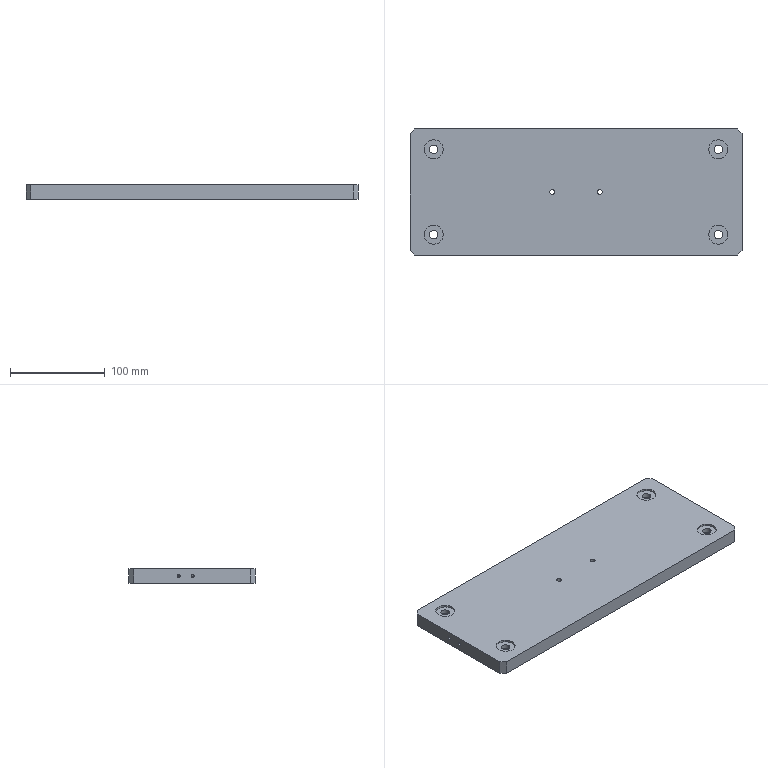Part | SolidWorks | features HoleWzd 3, Chamfer 1, Extrusion 1, ICE 1 | 1 solid | 54 faces | box 350 x 133 x 15 mm | volume 687021 mm3 | cylinder 32 | plane 18 | cone 4 | commonest cylinder face diameters 9 x8 15 x8 20 x8 3.3 x4 5 x4
STEP:
#1=CARTESIAN_POINT('',(-164.9,14.,-1.65));
#2=VERTEX_POINT('',#1);
#3=CARTESIAN_POINT('',(-164.9,14.,1.65));
#4=VERTEX_POINT('',#3);
#5=CARTESIAN_POINT('',(-164.9,14.,0.));
#6=DIRECTION('',(-1.,0.,0.));
#7=DIRECTION('',(0.,0.,1.));
#8=AXIS2_PLACEMENT_3D('',#5,#6,#7);
#9=CIRCLE('',#8,1.65);
#10=EDGE_CURVE('',#2,#4,#9,.T.);
#11=ORIENTED_EDGE('',*,*,#10,.F.);
#12=CARTESIAN_POINT('',(-175.,14.,-1.65));
#13=VERTEX_POINT('',#12);
#14=CARTESIAN_POINT('',(-175.,14.,-1.65));
#15=DIRECTION('',(-1.,0.,0.));
#16=VECTOR('',#15,1000.);
#17=LINE('',#14,#16);
#18=EDGE_CURVE('',#2,#13,#17,.T.);
#19=ORIENTED_EDGE('',*,*,#18,.T.);
#20=CARTESIAN_POINT('',(-175.,14.,1.65));
#21=VERTEX_POINT('',#20);
#22=CARTESIAN_POINT('',(-175.,14.,0.));
#23=DIRECTION('',(-1.,0.,0.));
#24=DIRECTION('',(0.,0.,1.));
#25=AXIS2_PLACEMENT_3D('',#22,#23,#24);
#26=CIRCLE('',#25,1.65);
#27=EDGE_CURVE('',#13,#21,#26,.T.);
#28=ORIENTED_EDGE('',*,*,#27,.T.);
#29=CARTESIAN_POINT('',(-175.,14.,1.65));
#30=DIRECTION('',(-1.,0.,0.));
#31=VECTOR('',#30,1000.);
#32=LINE('',#29,#31);
#33=EDGE_CURVE('',#4,#21,#32,.T.);
#34=ORIENTED_EDGE('',*,*,#33,.F.);
#35=EDGE_LOOP('',(#11,#19,#28,#34));
#36=FACE_OUTER_BOUND('',#35,.T.);
#37=CARTESIAN_POINT('',(-175.,14.,0.));
#38=DIRECTION('',(-1.,0.,0.));
#39=DIRECTION('',(0.,0.,1.));
#40=AXIS2_PLACEMENT_3D('',#37,#38,#39);
#41=CYLINDRICAL_SURFACE('',#40,1.65);
#42=ADVANCED_FACE('',(#36),#41,.F.);
#43=CARTESIAN_POINT('',(-163.909,14.,0.));
#44=VERTEX_POINT('',#43);
#45=CARTESIAN_POINT('',(-164.9,14.,1.65));
#46=DIRECTION('',(-0.515,0.,0.8572));
#47=VECTOR('',#46,1000.);
#48=LINE('',#45,#47);
#49=EDGE_CURVE('',#44,#4,#48,.T.);
#50=ORIENTED_EDGE('',*,*,#49,.F.);
#51=CARTESIAN_POINT('',(-164.9,14.,-1.65));
#52=DIRECTION('',(-0.515,0.,-0.8572));
#53=VECTOR('',#52,1000.);
#54=LINE('',#51,#53);
#55=EDGE_CURVE('',#44,#2,#54,.T.);
#56=ORIENTED_EDGE('',*,*,#55,.T.);
#57=ORIENTED_EDGE('',*,*,#10,.T.);
#58=EDGE_LOOP('',(#50,#56,#57));
#59=FACE_OUTER_BOUND('',#58,.T.);
#60=CARTESIAN_POINT('',(-164.9,14.,0.));
#61=DIRECTION('',(-1.,0.,0.));
#62=DIRECTION('',(0.,0.,1.));
#63=AXIS2_PLACEMENT_3D('',#60,#61,#62);
#64=CONICAL_SURFACE('',#63,1.65,1.03);
#65=ADVANCED_FACE('',(#59),#64,.F.);
#66=CARTESIAN_POINT('',(-164.9,-1.,-1.65));
#67=VERTEX_POINT('',#66);
#68=CARTESIAN_POINT('',(-164.9,-1.,1.65));
#69=VERTEX_POINT('',#68);
#70=CARTESIAN_POINT('',(-164.9,-1.,0.));
#71=DIRECTION('',(-1.,0.,0.));
#72=DIRECTION('',(0.,0.,1.));
#73=AXIS2_PLACEMENT_3D('',#70,#71,#72);
#74=CIRCLE('',#73,1.65);
#75=EDGE_CURVE('',#67,#69,#74,.T.);
#76=ORIENTED_EDGE('',*,*,#75,.F.);
#77=CARTESIAN_POINT('',(-175.,-1.,-1.65));
#78=VERTEX_POINT('',#77);
#79=CARTESIAN_POINT('',(-175.,-1.,-1.65));
#80=DIRECTION('',(-1.,0.,0.));
#81=VECTOR('',#80,1000.);
#82=LINE('',#79,#81);
#83=EDGE_CURVE('',#67,#78,#82,.T.);
#84=ORIENTED_EDGE('',*,*,#83,.T.);
#85=CARTESIAN_POINT('',(-175.,-1.,1.65));
#86=VERTEX_POINT('',#85);
#87=CARTESIAN_POINT('',(-175.,-1.,0.));
#88=DIRECTION('',(-1.,0.,0.));
#89=DIRECTION('',(0.,0.,1.));
#90=AXIS2_PLACEMENT_3D('',#87,#88,#89);
#91=CIRCLE('',#90,1.65);
#92=EDGE_CURVE('',#78,#86,#91,.T.);
#93=ORIENTED_EDGE('',*,*,#92,.T.);
#94=CARTESIAN_POINT('',(-175.,-1.,1.65));
#95=DIRECTION('',(-1.,0.,0.));
#96=VECTOR('',#95,1000.);
#97=LINE('',#94,#96);
#98=EDGE_CURVE('',#69,#86,#97,.T.);
#99=ORIENTED_EDGE('',*,*,#98,.F.);
#100=EDGE_LOOP('',(#76,#84,#93,#99));
#101=FACE_OUTER_BOUND('',#100,.T.);
#102=CARTESIAN_POINT('',(-175.,-1.,0.));
#103=DIRECTION('',(-1.,0.,0.));
#104=DIRECTION('',(0.,0.,1.));
#105=AXIS2_PLACEMENT_3D('',#102,#103,#104);
#106=CYLINDRICAL_SURFACE('',#105,1.65);
#107=ADVANCED_FACE('',(#101),#106,.F.);
#108=CARTESIAN_POINT('',(-163.909,-1.,0.));
#109=VERTEX_POINT('',#108);
#110=CARTESIAN_POINT('',(-164.9,-1.,1.65));
#111=DIRECTION('',(-0.515,0.,0.8572));
#112=VECTOR('',#111,1000.);
#113=LINE('',#110,#112);
#114=EDGE_CURVE('',#109,#69,#113,.T.);
#115=ORIENTED_EDGE('',*,*,#114,.F.);
#116=CARTESIAN_POINT('',(-164.9,-1.,-1.65));
#117=DIRECTION('',(-0.515,0.,-0.8572));
#118=VECTOR('',#117,1000.);
#119=LINE('',#116,#118);
#120=EDGE_CURVE('',#109,#67,#119,.T.);
#121=ORIENTED_EDGE('',*,*,#120,.T.);
#122=ORIENTED_EDGE('',*,*,#75,.T.);
#123=EDGE_LOOP('',(#115,#121,#122));
#124=FACE_OUTER_BOUND('',#123,.T.);
#125=CARTESIAN_POINT('',(-164.9,-1.,0.));
#126=DIRECTION('',(-1.,0.,0.));
#127=DIRECTION('',(0.,0.,1.));
#128=AXIS2_PLACEMENT_3D('',#125,#126,#127);
#129=CONICAL_SURFACE('',#128,1.65,1.03);
#130=ADVANCED_FACE('',(#124),#129,.F.);
#131=CARTESIAN_POINT('',(-160.,45.,5.5));
#132=VERTEX_POINT('',#131);
#133=CARTESIAN_POINT('',(-140.,45.,5.5));
#134=VERTEX_POINT('',#133);
#135=CARTESIAN_POINT('',(-150.,45.,5.5));
#136=DIRECTION('',(0.,0.,1.));
#137=DIRECTION('',(1.,0.,0.));
#138=AXIS2_PLACEMENT_3D('',#135,#136,#137);
#139=CIRCLE('',#138,10.);
#140=EDGE_CURVE('',#132,#134,#139,.T.);
#141=ORIENTED_EDGE('',*,*,#140,.F.);
#142=CARTESIAN_POINT('',(-160.,45.,7.5));
#143=VERTEX_POINT('',#142);
#144=CARTESIAN_POINT('',(-160.,45.,5.5));
#145=DIRECTION('',(0.,0.,1.));
#146=VECTOR('',#145,1000.);
#147=LINE('',#144,#146);
#148=EDGE_CURVE('',#132,#143,#147,.T.);
#149=ORIENTED_EDGE('',*,*,#148,.T.);
#150=CARTESIAN_POINT('',(-140.,45.,7.5));
#151=VERTEX_POINT('',#150);
#152=CARTESIAN_POINT('',(-150.,45.,7.5));
#153=DIRECTION('',(0.,0.,1.));
#154=DIRECTION('',(1.,0.,0.));
#155=AXIS2_PLACEMENT_3D('',#152,#153,#154);
#156=CIRCLE('',#155,10.);
#157=EDGE_CURVE('',#143,#151,#156,.T.);
#158=ORIENTED_EDGE('',*,*,#157,.T.);
#159=CARTESIAN_POINT('',(-140.,45.,5.5));
#160=DIRECTION('',(0.,0.,1.));
#161=VECTOR('',#160,1000.);
#162=LINE('',#159,#161);
#163=EDGE_CURVE('',#134,#151,#162,.T.);
#164=ORIENTED_EDGE('',*,*,#163,.F.);
#165=EDGE_LOOP('',(#141,#149,#158,#164));
#166=FACE_OUTER_BOUND('',#165,.T.);
#167=CARTESIAN_POINT('',(-150.,45.,5.5));
#168=DIRECTION('',(0.,0.,1.));
#169=DIRECTION('',(1.,0.,0.));
#170=AXIS2_PLACEMENT_3D('',#167,#168,#169);
#171=CYLINDRICAL_SURFACE('',#170,10.);
#172=ADVANCED_FACE('',(#166),#171,.F.);
#173=CARTESIAN_POINT('',(-160.,-45.,5.5));
#174=VERTEX_POINT('',#173);
#175=CARTESIAN_POINT('',(-140.,-45.,5.5));
#176=VERTEX_POINT('',#175);
#177=CARTESIAN_POINT('',(-150.,-45.,5.5));
#178=DIRECTION('',(0.,0.,1.));
#179=DIRECTION('',(-1.,0.,0.));
#180=AXIS2_PLACEMENT_3D('',#177,#178,#179);
#181=CIRCLE('',#180,10.);
#182=EDGE_CURVE('',#174,#176,#181,.T.);
#183=ORIENTED_EDGE('',*,*,#182,.F.);
#184=CARTESIAN_POINT('',(-160.,-45.,7.5));
#185=VERTEX_POINT('',#184);
#186=CARTESIAN_POINT('',(-160.,-45.,5.5));
#187=DIRECTION('',(0.,0.,1.));
#188=VECTOR('',#187,1000.);
#189=LINE('',#186,#188);
#190=EDGE_CURVE('',#174,#185,#189,.T.);
#191=ORIENTED_EDGE('',*,*,#190,.T.);
#192=CARTESIAN_POINT('',(-140.,-45.,7.5));
#193=VERTEX_POINT('',#192);
#194=CARTESIAN_POINT('',(-150.,-45.,7.5));
#195=DIRECTION('',(0.,0.,1.));
#196=DIRECTION('',(-1.,0.,0.));
#197=AXIS2_PLACEMENT_3D('',#194,#195,#196);
#198=CIRCLE('',#197,10.);
#199=EDGE_CURVE('',#185,#193,#198,.T.);
#200=ORIENTED_EDGE('',*,*,#199,.T.);
#201=CARTESIAN_POINT('',(-140.,-45.,5.5));
#202=DIRECTION('',(0.,0.,1.));
#203=VECTOR('',#202,1000.);
#204=LINE('',#201,#203);
#205=EDGE_CURVE('',#176,#193,#204,.T.);
#206=ORIENTED_EDGE('',*,*,#205,.F.);
#207=EDGE_LOOP('',(#183,#191,#200,#206));
#208=FACE_OUTER_BOUND('',#207,.T.);
#209=CARTESIAN_POINT('',(-150.,-45.,5.5));
#210=DIRECTION('',(0.,0.,1.));
#211=DIRECTION('',(1.,0.,0.));
#212=AXIS2_PLACEMENT_3D('',#209,#210,#211);
#213=CYLINDRICAL_SURFACE('',#212,10.);
#214=ADVANCED_FACE('',(#208),#213,.F.);
#215=CARTESIAN_POINT('',(140.,-45.,5.5));
#216=VERTEX_POINT('',#215);
#217=CARTESIAN_POINT('',(160.,-45.,5.5));
#218=VERTEX_POINT('',#217);
#219=CARTESIAN_POINT('',(150.,-45.,5.5));
#220=DIRECTION('',(0.,0.,1.));
#221=DIRECTION('',(1.,0.,0.));
#222=AXIS2_PLACEMENT_3D('',#219,#220,#221);
#223=CIRCLE('',#222,10.);
#224=EDGE_CURVE('',#216,#218,#223,.T.);
#225=ORIENTED_EDGE('',*,*,#224,.F.);
#226=CARTESIAN_POINT('',(140.,-45.,7.5));
#227=VERTEX_POINT('',#226);
#228=CARTESIAN_POINT('',(140.,-45.,5.5));
#229=DIRECTION('',(0.,0.,1.));
#230=VECTOR('',#229,1000.);
#231=LINE('',#228,#230);
#232=EDGE_CURVE('',#216,#227,#231,.T.);
#233=ORIENTED_EDGE('',*,*,#232,.T.);
#234=CARTESIAN_POINT('',(160.,-45.,7.5));
#235=VERTEX_POINT('',#234);
#236=CARTESIAN_POINT('',(150.,-45.,7.5));
#237=DIRECTION('',(0.,0.,1.));
#238=DIRECTION('',(1.,0.,0.));
#239=AXIS2_PLACEMENT_3D('',#236,#237,#238);
#240=CIRCLE('',#239,10.);
#241=EDGE_CURVE('',#227,#235,#240,.T.);
#242=ORIENTED_EDGE('',*,*,#241,.T.);
#243=CARTESIAN_POINT('',(160.,-45.,5.5));
#244=DIRECTION('',(0.,0.,1.));
#245=VECTOR('',#244,1000.);
#246=LINE('',#243,#245);
#247=EDGE_CURVE('',#218,#235,#246,.T.);
#248=ORIENTED_EDGE('',*,*,#247,.F.);
#249=EDGE_LOOP('',(#225,#233,#242,#248));
#250=FACE_OUTER_BOUND('',#249,.T.);
#251=CARTESIAN_POINT('',(150.,-45.,5.5));
#252=DIRECTION('',(0.,0.,1.));
#253=DIRECTION('',(1.,0.,0.));
#254=AXIS2_PLACEMENT_3D('',#251,#252,#253);
#255=CYLINDRICAL_SURFACE('',#254,10.);
#256=ADVANCED_FACE('',(#250),#255,.F.);
#257=CARTESIAN_POINT('',(140.,45.,5.5));
#258=VERTEX_POINT('',#257);
#259=CARTESIAN_POINT('',(160.,45.,5.5));
#260=VERTEX_POINT('',#259);
#261=CARTESIAN_POINT('',(150.,45.,5.5));
#262=DIRECTION('',(0.,0.,1.));
#263=DIRECTION('',(-1.,0.,0.));
#264=AXIS2_PLACEMENT_3D('',#261,#262,#263);
#265=CIRCLE('',#264,10.);
#266=EDGE_CURVE('',#258,#260,#265,.T.);
#267=ORIENTED_EDGE('',*,*,#266,.F.);
#268=CARTESIAN_POINT('',(140.,45.,7.5));
#269=VERTEX_POINT('',#268);
#270=CARTESIAN_POINT('',(140.,45.,5.5));
#271=DIRECTION('',(0.,0.,1.));
#272=VECTOR('',#271,1000.);
#273=LINE('',#270,#272);
#274=EDGE_CURVE('',#258,#269,#273,.T.);
#275=ORIENTED_EDGE('',*,*,#274,.T.);
#276=CARTESIAN_POINT('',(160.,45.,7.5));
#277=VERTEX_POINT('',#276);
#278=CARTESIAN_POINT('',(150.,45.,7.5));
#279=DIRECTION('',(0.,0.,1.));
#280=DIRECTION('',(-1.,0.,0.));
#281=AXIS2_PLACEMENT_3D('',#278,#279,#280);
#282=CIRCLE('',#281,10.);
#283=EDGE_CURVE('',#269,#277,#282,.T.);
#284=ORIENTED_EDGE('',*,*,#283,.T.);
#285=CARTESIAN_POINT('',(160.,45.,5.5));
#286=DIRECTION('',(0.,0.,1.));
#287=VECTOR('',#286,1000.);
#288=LINE('',#285,#287);
#289=EDGE_CURVE('',#260,#277,#288,.T.);
#290=ORIENTED_EDGE('',*,*,#289,.F.);
#291=EDGE_LOOP('',(#267,#275,#284,#290));
#292=FACE_OUTER_BOUND('',#291,.T.);
#293=CARTESIAN_POINT('',(150.,45.,5.5));
#294=DIRECTION('',(0.,0.,1.));
#295=DIRECTION('',(1.,0.,0.));
#296=AXIS2_PLACEMENT_3D('',#293,#294,#295);
#297=CYLINDRICAL_SURFACE('',#296,10.);
#298=ADVANCED_FACE('',(#292),#297,.F.);
#299=CARTESIAN_POINT('',(-27.5,0.,-7.5));
#300=VERTEX_POINT('',#299);
#301=CARTESIAN_POINT('',(-22.5,0.,-7.5));
#302=VERTEX_POINT('',#301);
#303=CARTESIAN_POINT('',(-25.,0.,-7.5));
#304=DIRECTION('',(0.,0.,1.));
#305=DIRECTION('',(1.,0.,0.));
#306=AXIS2_PLACEMENT_3D('',#303,#304,#305);
#307=CIRCLE('',#306,2.5);
#308=EDGE_CURVE('',#300,#302,#307,.T.);
#309=ORIENTED_EDGE('',*,*,#308,.F.);
#310=CARTESIAN_POINT('',(-27.5,0.,7.5));
#311=VERTEX_POINT('',#310);
#312=CARTESIAN_POINT('',(-27.5,0.,7.5));
#313=DIRECTION('',(0.,0.,1.));
#314=VECTOR('',#313,1000.);
#315=LINE('',#312,#314);
#316=EDGE_CURVE('',#300,#311,#315,.T.);
#317=ORIENTED_EDGE('',*,*,#316,.T.);
#318=CARTESIAN_POINT('',(-22.5,0.,7.5));
#319=VERTEX_POINT('',#318);
#320=CARTESIAN_POINT('',(-25.,0.,7.5));
#321=DIRECTION('',(0.,0.,1.));
#322=DIRECTION('',(1.,0.,0.));
#323=AXIS2_PLACEMENT_3D('',#320,#321,#322);
#324=CIRCLE('',#323,2.5);
#325=EDGE_CURVE('',#311,#319,#324,.T.);
#326=ORIENTED_EDGE('',*,*,#325,.T.);
#327=CARTESIAN_POINT('',(-22.5,0.,7.5));
#328=DIRECTION('',(0.,0.,1.));
#329=VECTOR('',#328,1000.);
#330=LINE('',#327,#329);
#331=EDGE_CURVE('',#302,#319,#330,.T.);
#332=ORIENTED_EDGE('',*,*,#331,.F.);
#333=EDGE_LOOP('',(#309,#317,#326,#332));
#334=FACE_OUTER_BOUND('',#333,.T.);
#335=CARTESIAN_POINT('',(-25.,0.,7.5));
#336=DIRECTION('',(0.,0.,1.));
#337=DIRECTION('',(1.,0.,0.));
#338=AXIS2_PLACEMENT_3D('',#335,#336,#337);
#339=CYLINDRICAL_SURFACE('',#338,2.5);
#340=ADVANCED_FACE('',(#334),#339,.F.);
#341=CARTESIAN_POINT('',(22.5,0.,-7.5));
#342=VERTEX_POINT('',#341);
#343=CARTESIAN_POINT('',(27.5,0.,-7.5));
#344=VERTEX_POINT('',#343);
#345=CARTESIAN_POINT('',(25.,0.,-7.5));
#346=DIRECTION('',(0.,0.,1.));
#347=DIRECTION('',(1.,0.,0.));
#348=AXIS2_PLACEMENT_3D('',#345,#346,#347);
#349=CIRCLE('',#348,2.5);
#350=EDGE_CURVE('',#342,#344,#349,.T.);
#351=ORIENTED_EDGE('',*,*,#350,.F.);
#352=CARTESIAN_POINT('',(22.5,0.,7.5));
#353=VERTEX_POINT('',#352);
#354=CARTESIAN_POINT('',(22.5,0.,7.5));
#355=DIRECTION('',(0.,0.,1.));
#356=VECTOR('',#355,1000.);
#357=LINE('',#354,#356);
#358=EDGE_CURVE('',#342,#353,#357,.T.);
#359=ORIENTED_EDGE('',*,*,#358,.T.);
#360=CARTESIAN_POINT('',(27.5,0.,7.5));
#361=VERTEX_POINT('',#360);
#362=CARTESIAN_POINT('',(25.,0.,7.5));
#363=DIRECTION('',(0.,0.,1.));
#364=DIRECTION('',(1.,0.,0.));
#365=AXIS2_PLACEMENT_3D('',#362,#363,#364);
#366=CIRCLE('',#365,2.5);
#367=EDGE_CURVE('',#353,#361,#366,.T.);
#368=ORIENTED_EDGE('',*,*,#367,.T.);
#369=CARTESIAN_POINT('',(27.5,0.,7.5));
#370=DIRECTION('',(0.,0.,1.));
#371=VECTOR('',#370,1000.);
#372=LINE('',#369,#371);
#373=EDGE_CURVE('',#344,#361,#372,.T.);
#374=ORIENTED_EDGE('',*,*,#373,.F.);
#375=EDGE_LOOP('',(#351,#359,#368,#374));
#376=FACE_OUTER_BOUND('',#375,.T.);
#377=CARTESIAN_POINT('',(25.,0.,7.5));
#378=DIRECTION('',(0.,0.,1.));
#379=DIRECTION('',(1.,0.,0.));
#380=AXIS2_PLACEMENT_3D('',#377,#378,#379);
#381=CYLINDRICAL_SURFACE('',#380,2.5);
#382=ADVANCED_FACE('',(#376),#381,.F.);
#383=CARTESIAN_POINT('',(157.5,45.,1.1));
#384=VERTEX_POINT('',#383);
#385=CARTESIAN_POINT('',(142.5,45.,1.1));
#386=VERTEX_POINT('',#385);
#387=CARTESIAN_POINT('',(150.,45.,1.1));
#388=DIRECTION('',(0.,0.,-1.));
#389=DIRECTION('',(-1.,0.,0.));
#390=AXIS2_PLACEMENT_3D('',#387,#388,#389);
#391=CIRCLE('',#390,7.5);
#392=EDGE_CURVE('',#384,#386,#391,.T.);
#393=ORIENTED_EDGE('',*,*,#392,.F.);
#394=CARTESIAN_POINT('',(157.5,45.,-7.5));
#395=VERTEX_POINT('',#394);
#396=CARTESIAN_POINT('',(157.5,45.,-7.5));
#397=DIRECTION('',(0.,0.,-1.));
#398=VECTOR('',#397,1000.);
#399=LINE('',#396,#398);
#400=EDGE_CURVE('',#384,#395,#399,.T.);
#401=ORIENTED_EDGE('',*,*,#400,.T.);
#402=CARTESIAN_POINT('',(142.5,45.,-7.5));
#403=VERTEX_POINT('',#402);
#404=CARTESIAN_POINT('',(150.,45.,-7.5));
#405=DIRECTION('',(0.,0.,-1.));
#406=DIRECTION('',(-1.,0.,0.));
#407=AXIS2_PLACEMENT_3D('',#404,#405,#406);
#408=CIRCLE('',#407,7.5);
#409=EDGE_CURVE('',#395,#403,#408,.T.);
#410=ORIENTED_EDGE('',*,*,#409,.T.);
#411=CARTESIAN_POINT('',(142.5,45.,-7.5));
#412=DIRECTION('',(0.,0.,-1.));
#413=VECTOR('',#412,1000.);
#414=LINE('',#411,#413);
#415=EDGE_CURVE('',#386,#403,#414,.T.);
#416=ORIENTED_EDGE('',*,*,#415,.F.);
#417=EDGE_LOOP('',(#393,#401,#410,#416));
#418=FACE_OUTER_BOUND('',#417,.T.);
#419=CARTESIAN_POINT('',(150.,45.,-7.5));
#420=DIRECTION('',(0.,0.,-1.));
#421=DIRECTION('',(-1.,0.,0.));
#422=AXIS2_PLACEMENT_3D('',#419,#420,#421);
#423=CYLINDRICAL_SURFACE('',#422,7.5);
#424=ADVANCED_FACE('',(#418),#423,.F.);
#425=CARTESIAN_POINT('',(145.5,45.,5.5));
#426=VERTEX_POINT('',#425);
#427=CARTESIAN_POINT('',(154.5,45.,5.5));
#428=VERTEX_POINT('',#427);
#429=CARTESIAN_POINT('',(150.,45.,5.5));
#430=DIRECTION('',(0.,0.,1.));
#431=DIRECTION('',(-1.,0.,0.));
#432=AXIS2_PLACEMENT_3D('',#429,#430,#431);
#433=CIRCLE('',#432,4.5);
#434=EDGE_CURVE('',#426,#428,#433,.T.);
#435=ORIENTED_EDGE('',*,*,#434,.T.);
#436=CARTESIAN_POINT('',(154.5,45.,1.1));
#437=VERTEX_POINT('',#436);
#438=CARTESIAN_POINT('',(154.5,45.,-7.5));
#439=DIRECTION('',(0.,0.,-1.));
#440=VECTOR('',#439,1000.);
#441=LINE('',#438,#440);
#442=EDGE_CURVE('',#428,#437,#441,.T.);
#443=ORIENTED_EDGE('',*,*,#442,.T.);
#444=CARTESIAN_POINT('',(145.5,45.,1.1));
#445=VERTEX_POINT('',#444);
#446=CARTESIAN_POINT('',(150.,45.,1.1));
#447=DIRECTION('',(0.,0.,-1.));
#448=DIRECTION('',(-1.,0.,0.));
#449=AXIS2_PLACEMENT_3D('',#446,#447,#448);
#450=CIRCLE('',#449,4.5);
#451=EDGE_CURVE('',#437,#445,#450,.T.);
#452=ORIENTED_EDGE('',*,*,#451,.T.);
#453=CARTESIAN_POINT('',(145.5,45.,-7.5));
#454=DIRECTION('',(0.,0.,-1.));
#455=VECTOR('',#454,1000.);
#456=LINE('',#453,#455);
#457=EDGE_CURVE('',#426,#445,#456,.T.);
#458=ORIENTED_EDGE('',*,*,#457,.F.);
#459=EDGE_LOOP('',(#435,#443,#452,#458));
#460=FACE_OUTER_BOUND('',#459,.T.);
#461=CARTESIAN_POINT('',(150.,45.,-7.5));
#462=DIRECTION('',(0.,0.,-1.));
#463=DIRECTION('',(-1.,0.,0.));
#464=AXIS2_PLACEMENT_3D('',#461,#462,#463);
#465=CYLINDRICAL_SURFACE('',#464,4.5);
#466=ADVANCED_FACE('',(#460),#465,.F.);
#467=CARTESIAN_POINT('',(157.5,-45.,1.1));
#468=VERTEX_POINT('',#467);
#469=CARTESIAN_POINT('',(142.5,-45.,1.1));
#470=VERTEX_POINT('',#469);
#471=CARTESIAN_POINT('',(150.,-45.,1.1));
#472=DIRECTION('',(0.,0.,-1.));
#473=DIRECTION('',(-1.,0.,0.));
#474=AXIS2_PLACEMENT_3D('',#471,#472,#473);
#475=CIRCLE('',#474,7.5);
#476=EDGE_CURVE('',#468,#470,#475,.T.);
#477=ORIENTED_EDGE('',*,*,#476,.F.);
#478=CARTESIAN_POINT('',(157.5,-45.,-7.5));
#479=VERTEX_POINT('',#478);
#480=CARTESIAN_POINT('',(157.5,-45.,-7.5));
#481=DIRECTION('',(0.,0.,-1.));
#482=VECTOR('',#481,1000.);
#483=LINE('',#480,#482);
#484=EDGE_CURVE('',#468,#479,#483,.T.);
#485=ORIENTED_EDGE('',*,*,#484,.T.);
#486=CARTESIAN_POINT('',(142.5,-45.,-7.5));
#487=VERTEX_POINT('',#486);
#488=CARTESIAN_POINT('',(150.,-45.,-7.5));
#489=DIRECTION('',(0.,0.,-1.));
#490=DIRECTION('',(-1.,0.,0.));
#491=AXIS2_PLACEMENT_3D('',#488,#489,#490);
#492=CIRCLE('',#491,7.5);
#493=EDGE_CURVE('',#479,#487,#492,.T.);
#494=ORIENTED_EDGE('',*,*,#493,.T.);
#495=CARTESIAN_POINT('',(142.5,-45.,-7.5));
#496=DIRECTION('',(0.,0.,-1.));
#497=VECTOR('',#496,1000.);
#498=LINE('',#495,#497);
#499=EDGE_CURVE('',#470,#487,#498,.T.);
#500=ORIENTED_EDGE('',*,*,#499,.F.);
#501=EDGE_LOOP('',(#477,#485,#494,#500));
#502=FACE_OUTER_BOUND('',#501,.T.);
#503=CARTESIAN_POINT('',(150.,-45.,-7.5));
#504=DIRECTION('',(0.,0.,-1.));
#505=DIRECTION('',(-1.,0.,0.));
#506=AXIS2_PLACEMENT_3D('',#503,#504,#505);
#507=CYLINDRICAL_SURFACE('',#506,7.5);
#508=ADVANCED_FACE('',(#502),#507,.F.);
#509=CARTESIAN_POINT('',(-142.5,-45.,1.1));
#510=VERTEX_POINT('',#509);
#511=CARTESIAN_POINT('',(-157.5,-45.,1.1));
#512=VERTEX_POINT('',#511);
#513=CARTESIAN_POINT('',(-150.,-45.,1.1));
#514=DIRECTION('',(0.,0.,-1.));
#515=DIRECTION('',(-1.,0.,0.));
#516=AXIS2_PLACEMENT_3D('',#513,#514,#515);
#517=CIRCLE('',#516,7.5);
#518=EDGE_CURVE('',#510,#512,#517,.T.);
#519=ORIENTED_EDGE('',*,*,#518,.F.);
#520=CARTESIAN_POINT('',(-142.5,-45.,-7.5));
#521=VERTEX_POINT('',#520);
#522=CARTESIAN_POINT('',(-142.5,-45.,-7.5));
#523=DIRECTION('',(0.,0.,-1.));
#524=VECTOR('',#523,1000.);
#525=LINE('',#522,#524);
#526=EDGE_CURVE('',#510,#521,#525,.T.);
#527=ORIENTED_EDGE('',*,*,#526,.T.);
#528=CARTESIAN_POINT('',(-157.5,-45.,-7.5));
#529=VERTEX_POINT('',#528);
#530=CARTESIAN_POINT('',(-150.,-45.,-7.5));
#531=DIRECTION('',(0.,0.,-1.));
#532=DIRECTION('',(-1.,0.,0.));
#533=AXIS2_PLACEMENT_3D('',#530,#531,#532);
#534=CIRCLE('',#533,7.5);
#535=EDGE_CURVE('',#521,#529,#534,.T.);
#536=ORIENTED_EDGE('',*,*,#535,.T.);
#537=CARTESIAN_POINT('',(-157.5,-45.,-7.5));
#538=DIRECTION('',(0.,0.,-1.));
#539=VECTOR('',#538,1000.);
#540=LINE('',#537,#539);
#541=EDGE_CURVE('',#512,#529,#540,.T.);
#542=ORIENTED_EDGE('',*,*,#541,.F.);
#543=EDGE_LOOP('',(#519,#527,#536,#542));
#544=FACE_OUTER_BOUND('',#543,.T.);
#545=CARTESIAN_POINT('',(-150.,-45.,-7.5));
#546=DIRECTION('',(0.,0.,-1.));
#547=DIRECTION('',(-1.,0.,0.));
#548=AXIS2_PLACEMENT_3D('',#545,#546,#547);
#549=CYLINDRICAL_SURFACE('',#548,7.5);
#550=ADVANCED_FACE('',(#544),#549,.F.);
#551=CARTESIAN_POINT('',(-154.5,-45.,5.5));
#552=VERTEX_POINT('',#551);
#553=CARTESIAN_POINT('',(-145.5,-45.,5.5));
#554=VERTEX_POINT('',#553);
#555=CARTESIAN_POINT('',(-150.,-45.,5.5));
#556=DIRECTION('',(0.,0.,1.));
#557=DIRECTION('',(-1.,0.,0.));
#558=AXIS2_PLACEMENT_3D('',#555,#556,#557);
#559=CIRCLE('',#558,4.5);
#560=EDGE_CURVE('',#552,#554,#559,.T.);
#561=ORIENTED_EDGE('',*,*,#560,.T.);
#562=CARTESIAN_POINT('',(-145.5,-45.,1.1));
#563=VERTEX_POINT('',#562);
#564=CARTESIAN_POINT('',(-145.5,-45.,-7.5));
#565=DIRECTION('',(0.,0.,-1.));
#566=VECTOR('',#565,1000.);
#567=LINE('',#564,#566);
#568=EDGE_CURVE('',#554,#563,#567,.T.);
#569=ORIENTED_EDGE('',*,*,#568,.T.);
#570=CARTESIAN_POINT('',(-154.5,-45.,1.1));
#571=VERTEX_POINT('',#570);
#572=CARTESIAN_POINT('',(-150.,-45.,1.1));
#573=DIRECTION('',(0.,0.,-1.));
#574=DIRECTION('',(-1.,0.,0.));
#575=AXIS2_PLACEMENT_3D('',#572,#573,#574);
#576=CIRCLE('',#575,4.5);
#577=EDGE_CURVE('',#563,#571,#576,.T.);
#578=ORIENTED_EDGE('',*,*,#577,.T.);
#579=CARTESIAN_POINT('',(-154.5,-45.,-7.5));
#580=DIRECTION('',(0.,0.,-1.));
#581=VECTOR('',#580,1000.);
#582=LINE('',#579,#581);
#583=EDGE_CURVE('',#552,#571,#582,.T.);
#584=ORIENTED_EDGE('',*,*,#583,.F.);
#585=EDGE_LOOP('',(#561,#569,#578,#584));
#586=FACE_OUTER_BOUND('',#585,.T.);
#587=CARTESIAN_POINT('',(-150.,-45.,-7.5));
#588=DIRECTION('',(0.,0.,-1.));
#589=DIRECTION('',(-1.,0.,0.));
#590=AXIS2_PLACEMENT_3D('',#587,#588,#589);
#591=CYLINDRICAL_SURFACE('',#590,4.5);
#592=ADVANCED_FACE('',(#586),#591,.F.);
#593=CARTESIAN_POINT('',(-142.5,45.,1.1));
#594=VERTEX_POINT('',#593);
#595=CARTESIAN_POINT('',(-157.5,45.,1.1));
#596=VERTEX_POINT('',#595);
#597=CARTESIAN_POINT('',(-150.,45.,1.1));
#598=DIRECTION('',(0.,0.,-1.));
#599=DIRECTION('',(-1.,0.,0.));
#600=AXIS2_PLACEMENT_3D('',#597,#598,#599);
#601=CIRCLE('',#600,7.5);
#602=EDGE_CURVE('',#594,#596,#601,.T.);
#603=ORIENTED_EDGE('',*,*,#602,.F.);
#604=CARTESIAN_POINT('',(-142.5,45.,-7.5));
#605=VERTEX_POINT('',#604);
#606=CARTESIAN_POINT('',(-142.5,45.,-7.5));
#607=DIRECTION('',(0.,0.,-1.));
#608=VECTOR('',#607,1000.);
#609=LINE('',#606,#608);
#610=EDGE_CURVE('',#594,#605,#609,.T.);
#611=ORIENTED_EDGE('',*,*,#610,.T.);
#612=CARTESIAN_POINT('',(-157.5,45.,-7.5));
#613=VERTEX_POINT('',#612);
#614=CARTESIAN_POINT('',(-150.,45.,-7.5));
#615=DIRECTION('',(0.,0.,-1.));
#616=DIRECTION('',(-1.,0.,0.));
#617=AXIS2_PLACEMENT_3D('',#614,#615,#616);
#618=CIRCLE('',#617,7.5);
#619=EDGE_CURVE('',#605,#613,#618,.T.);
#620=ORIENTED_EDGE('',*,*,#619,.T.);
#621=CARTESIAN_POINT('',(-157.5,45.,-7.5));
#622=DIRECTION('',(0.,0.,-1.));
#623=VECTOR('',#622,1000.);
#624=LINE('',#621,#623);
#625=EDGE_CURVE('',#596,#613,#624,.T.);
#626=ORIENTED_EDGE('',*,*,#625,.F.);
#627=EDGE_LOOP('',(#603,#611,#620,#626));
#628=FACE_OUTER_BOUND('',#627,.T.);
#629=CARTESIAN_POINT('',(-150.,45.,-7.5));
#630=DIRECTION('',(0.,0.,-1.));
#631=DIRECTION('',(-1.,0.,0.));
#632=AXIS2_PLACEMENT_3D('',#629,#630,#631);
#633=CYLINDRICAL_SURFACE('',#632,7.5);
#634=ADVANCED_FACE('',(#628),#633,.F.);
#635=CARTESIAN_POINT('',(154.5,-45.,5.5));
#636=VERTEX_POINT('',#635);
#637=CARTESIAN_POINT('',(145.5,-45.,5.5));
#638=VERTEX_POINT('',#637);
#639=CARTESIAN_POINT('',(150.,-45.,5.5));
#640=DIRECTION('',(0.,0.,-1.));
#641=DIRECTION('',(1.,0.,0.));
#642=AXIS2_PLACEMENT_3D('',#639,#640,#641);
#643=CIRCLE('',#642,4.5);
#644=EDGE_CURVE('',#636,#638,#643,.T.);
#645=ORIENTED_EDGE('',*,*,#644,.F.);
#646=CARTESIAN_POINT('',(154.5,-45.,1.1));
#647=VERTEX_POINT('',#646);
#648=CARTESIAN_POINT('',(154.5,-45.,-7.5));
#649=DIRECTION('',(0.,0.,-1.));
#650=VECTOR('',#649,1000.);
#651=LINE('',#648,#650);
#652=EDGE_CURVE('',#636,#647,#651,.T.);
#653=ORIENTED_EDGE('',*,*,#652,.T.);
#654=CARTESIAN_POINT('',(145.5,-45.,1.1));
#655=VERTEX_POINT('',#654);
#656=CARTESIAN_POINT('',(150.,-45.,1.1));
#657=DIRECTION('',(0.,0.,-1.));
#658=DIRECTION('',(-1.,0.,0.));
#659=AXIS2_PLACEMENT_3D('',#656,#657,#658);
#660=CIRCLE('',#659,4.5);
#661=EDGE_CURVE('',#647,#655,#660,.T.);
#662=ORIENTED_EDGE('',*,*,#661,.T.);
#663=CARTESIAN_POINT('',(145.5,-45.,-7.5));
#664=DIRECTION('',(0.,0.,-1.));
#665=VECTOR('',#664,1000.);
#666=LINE('',#663,#665);
#667=EDGE_CURVE('',#638,#655,#666,.T.);
#668=ORIENTED_EDGE('',*,*,#667,.F.);
#669=EDGE_LOOP('',(#645,#653,#662,#668));
#670=FACE_OUTER_BOUND('',#669,.T.);
#671=CARTESIAN_POINT('',(150.,-45.,-7.5));
#672=DIRECTION('',(0.,0.,-1.));
#673=DIRECTION('',(-1.,0.,0.));
#674=AXIS2_PLACEMENT_3D('',#671,#672,#673);
#675=CYLINDRICAL_SURFACE('',#674,4.5);
#676=ADVANCED_FACE('',(#670),#675,.F.);
#677=CARTESIAN_POINT('',(-145.5,45.,5.5));
#678=VERTEX_POINT('',#677);
#679=CARTESIAN_POINT('',(-154.5,45.,5.5));
#680=VERTEX_POINT('',#679);
#681=CARTESIAN_POINT('',(-150.,45.,5.5));
#682=DIRECTION('',(0.,0.,-1.));
#683=DIRECTION('',(1.,0.,0.));
#684=AXIS2_PLACEMENT_3D('',#681,#682,#683);
#685=CIRCLE('',#684,4.5);
#686=EDGE_CURVE('',#678,#680,#685,.T.);
#687=ORIENTED_EDGE('',*,*,#686,.F.);
#688=CARTESIAN_POINT('',(-145.5,45.,1.1));
#689=VERTEX_POINT('',#688);
#690=CARTESIAN_POINT('',(-145.5,45.,-7.5));
#691=DIRECTION('',(0.,0.,-1.));
#692=VECTOR('',#691,1000.);
#693=LINE('',#690,#692);
#694=EDGE_CURVE('',#678,#689,#693,.T.);
#695=ORIENTED_EDGE('',*,*,#694,.T.);
#696=CARTESIAN_POINT('',(-154.5,45.,1.1));
#697=VERTEX_POINT('',#696);
#698=CARTESIAN_POINT('',(-150.,45.,1.1));
#699=DIRECTION('',(0.,0.,-1.));
#700=DIRECTION('',(-1.,0.,0.));
#701=AXIS2_PLACEMENT_3D('',#698,#699,#700);
#702=CIRCLE('',#701,4.5);
#703=EDGE_CURVE('',#689,#697,#702,.T.);
#704=ORIENTED_EDGE('',*,*,#703,.T.);
#705=CARTESIAN_POINT('',(-154.5,45.,-7.5));
#706=DIRECTION('',(0.,0.,-1.));
#707=VECTOR('',#706,1000.);
#708=LINE('',#705,#707);
#709=EDGE_CURVE('',#680,#697,#708,.T.);
#710=ORIENTED_EDGE('',*,*,#709,.F.);
#711=EDGE_LOOP('',(#687,#695,#704,#710));
#712=FACE_OUTER_BOUND('',#711,.T.);
#713=CARTESIAN_POINT('',(-150.,45.,-7.5));
#714=DIRECTION('',(0.,0.,-1.));
#715=DIRECTION('',(-1.,0.,0.));
#716=AXIS2_PLACEMENT_3D('',#713,#714,#715);
#717=CYLINDRICAL_SURFACE('',#716,4.5);
#718=ADVANCED_FACE('',(#712),#717,.F.);
#719=ORIENTED_EDGE('',*,*,#694,.F.);
#720=CARTESIAN_POINT('',(-150.,45.,5.5));
#721=DIRECTION('',(0.,0.,-1.));
#722=DIRECTION('',(1.,0.,0.));
#723=AXIS2_PLACEMENT_3D('',#720,#721,#722);
#724=CIRCLE('',#723,4.5);
#725=EDGE_CURVE('',#680,#678,#724,.T.);
#726=ORIENTED_EDGE('',*,*,#725,.F.);
#727=ORIENTED_EDGE('',*,*,#709,.T.);
#728=CARTESIAN_POINT('',(-150.,45.,1.1));
#729=DIRECTION('',(0.,0.,-1.));
#730=DIRECTION('',(-1.,0.,0.));
#731=AXIS2_PLACEMENT_3D('',#728,#729,#730);
#732=CIRCLE('',#731,4.5);
#733=EDGE_CURVE('',#697,#689,#732,.T.);
#734=ORIENTED_EDGE('',*,*,#733,.T.);
#735=EDGE_LOOP('',(#719,#726,#727,#734));
#736=FACE_OUTER_BOUND('',#735,.T.);
#737=CARTESIAN_POINT('',(-150.,45.,-7.5));
#738=DIRECTION('',(0.,0.,-1.));
#739=DIRECTION('',(-1.,0.,0.));
#740=AXIS2_PLACEMENT_3D('',#737,#738,#739);
#741=CYLINDRICAL_SURFACE('',#740,4.5);
#742=ADVANCED_FACE('',(#736),#741,.F.);
#743=ORIENTED_EDGE('',*,*,#652,.F.);
#744=CARTESIAN_POINT('',(150.,-45.,5.5));
#745=DIRECTION('',(0.,0.,-1.));
#746=DIRECTION('',(1.,0.,0.));
#747=AXIS2_PLACEMENT_3D('',#744,#745,#746);
#748=CIRCLE('',#747,4.5);
#749=EDGE_CURVE('',#638,#636,#748,.T.);
#750=ORIENTED_EDGE('',*,*,#749,.F.);
#751=ORIENTED_EDGE('',*,*,#667,.T.);
#752=CARTESIAN_POINT('',(150.,-45.,1.1));
#753=DIRECTION('',(0.,0.,-1.));
#754=DIRECTION('',(-1.,0.,0.));
#755=AXIS2_PLACEMENT_3D('',#752,#753,#754);
#756=CIRCLE('',#755,4.5);
#757=EDGE_CURVE('',#655,#647,#756,.T.);
#758=ORIENTED_EDGE('',*,*,#757,.T.);
#759=EDGE_LOOP('',(#743,#750,#751,#758));
#760=FACE_OUTER_BOUND('',#759,.T.);
#761=CARTESIAN_POINT('',(150.,-45.,-7.5));
#762=DIRECTION('',(0.,0.,-1.));
#763=DIRECTION('',(-1.,0.,0.));
#764=AXIS2_PLACEMENT_3D('',#761,#762,#763);
#765=CYLINDRICAL_SURFACE('',#764,4.5);
#766=ADVANCED_FACE('',(#760),#765,.F.);
#767=CARTESIAN_POINT('',(175.,-61.5,-7.5));
#768=VERTEX_POINT('',#767);
#769=CARTESIAN_POINT('',(175.,61.5,-7.5));
#770=VERTEX_POINT('',#769);
#771=CARTESIAN_POINT('',(175.,-66.5,-7.5));
#772=DIRECTION('',(0.,1.,0.));
#773=VECTOR('',#772,1000.);
#774=LINE('',#771,#773);
#775=EDGE_CURVE('',#768,#770,#774,.T.);
#776=ORIENTED_EDGE('',*,*,#775,.T.);
#777=CARTESIAN_POINT('',(175.,61.5,7.5));
#778=VERTEX_POINT('',#777);
#779=CARTESIAN_POINT('',(175.,61.5,7.5));
#780=DIRECTION('',(0.,0.,1.));
#781=VECTOR('',#780,1000.);
#782=LINE('',#779,#781);
#783=EDGE_CURVE('',#770,#778,#782,.T.);
#784=ORIENTED_EDGE('',*,*,#783,.T.);
#785=CARTESIAN_POINT('',(175.,-61.5,7.5));
#786=VERTEX_POINT('',#785);
#787=CARTESIAN_POINT('',(175.,-66.5,7.5));
#788=DIRECTION('',(0.,1.,0.));
#789=VECTOR('',#788,1000.);
#790=LINE('',#787,#789);
#791=EDGE_CURVE('',#786,#778,#790,.T.);
#792=ORIENTED_EDGE('',*,*,#791,.F.);
#793=CARTESIAN_POINT('',(175.,-61.5,7.5));
#794=DIRECTION('',(0.,0.,-1.));
#795=VECTOR('',#794,1000.);
#796=LINE('',#793,#795);
#797=EDGE_CURVE('',#786,#768,#796,.T.);
#798=ORIENTED_EDGE('',*,*,#797,.T.);
#799=EDGE_LOOP('',(#776,#784,#792,#798));
#800=FACE_OUTER_BOUND('',#799,.T.);
#801=CARTESIAN_POINT('',(175.,-66.5,7.5));
#802=DIRECTION('',(-1.,0.,0.));
#803=DIRECTION('',(0.,0.,1.));
#804=AXIS2_PLACEMENT_3D('',#801,#802,#803);
#805=PLANE('',#804);
#806=ADVANCED_FACE('',(#800),#805,.F.);
#807=CARTESIAN_POINT('',(170.,66.5,7.5));
#808=VERTEX_POINT('',#807);
#809=CARTESIAN_POINT('',(-170.,66.5,7.5));
#810=VERTEX_POINT('',#809);
#811=CARTESIAN_POINT('',(-175.,66.5,7.5));
#812=DIRECTION('',(-1.,0.,0.));
#813=VECTOR('',#812,1000.);
#814=LINE('',#811,#813);
#815=EDGE_CURVE('',#808,#810,#814,.T.);
#816=ORIENTED_EDGE('',*,*,#815,.F.);
#817=CARTESIAN_POINT('',(170.,66.5,-7.5));
#818=VERTEX_POINT('',#817);
#819=CARTESIAN_POINT('',(170.,66.5,7.5));
#820=DIRECTION('',(0.,0.,-1.));
#821=VECTOR('',#820,1000.);
#822=LINE('',#819,#821);
#823=EDGE_CURVE('',#808,#818,#822,.T.);
#824=ORIENTED_EDGE('',*,*,#823,.T.);
#825=CARTESIAN_POINT('',(-170.,66.5,-7.5));
#826=VERTEX_POINT('',#825);
#827=CARTESIAN_POINT('',(-175.,66.5,-7.5));
#828=DIRECTION('',(-1.,0.,0.));
#829=VECTOR('',#828,1000.);
#830=LINE('',#827,#829);
#831=EDGE_CURVE('',#818,#826,#830,.T.);
#832=ORIENTED_EDGE('',*,*,#831,.T.);
#833=CARTESIAN_POINT('',(-170.,66.5,7.5));
#834=DIRECTION('',(0.,0.,1.));
#835=VECTOR('',#834,1000.);
#836=LINE('',#833,#835);
#837=EDGE_CURVE('',#826,#810,#836,.T.);
#838=ORIENTED_EDGE('',*,*,#837,.T.);
#839=EDGE_LOOP('',(#816,#824,#832,#838));
#840=FACE_OUTER_BOUND('',#839,.T.);
#841=CARTESIAN_POINT('',(-175.,66.5,7.5));
#842=DIRECTION('',(0.,-1.,0.));
#843=DIRECTION('',(0.,0.,-1.));
#844=AXIS2_PLACEMENT_3D('',#841,#842,#843);
#845=PLANE('',#844);
#846=ADVANCED_FACE('',(#840),#845,.F.);
#847=CARTESIAN_POINT('',(-175.,14.,0.));
#848=DIRECTION('',(-1.,0.,0.));
#849=DIRECTION('',(0.,0.,1.));
#850=AXIS2_PLACEMENT_3D('',#847,#848,#849);
#851=CIRCLE('',#850,1.65);
#852=EDGE_CURVE('',#21,#13,#851,.T.);
#853=ORIENTED_EDGE('',*,*,#852,.F.);
#854=ORIENTED_EDGE('',*,*,#27,.F.);
#855=EDGE_LOOP('',(#853,#854));
#856=FACE_BOUND('',#855,.T.);
#857=CARTESIAN_POINT('',(-175.,-1.,0.));
#858=DIRECTION('',(-1.,0.,0.));
#859=DIRECTION('',(0.,0.,1.));
#860=AXIS2_PLACEMENT_3D('',#857,#858,#859);
#861=CIRCLE('',#860,1.65);
#862=EDGE_CURVE('',#86,#78,#861,.T.);
#863=ORIENTED_EDGE('',*,*,#862,.F.);
#864=ORIENTED_EDGE('',*,*,#92,.F.);
#865=EDGE_LOOP('',(#863,#864));
#866=FACE_BOUND('',#865,.T.);
#867=CARTESIAN_POINT('',(-175.,61.5,7.5));
#868=VERTEX_POINT('',#867);
#869=CARTESIAN_POINT('',(-175.,-61.5,7.5));
#870=VERTEX_POINT('',#869);
#871=CARTESIAN_POINT('',(-175.,-66.5,7.5));
#872=DIRECTION('',(0.,-1.,0.));
#873=VECTOR('',#872,1000.);
#874=LINE('',#871,#873);
#875=EDGE_CURVE('',#868,#870,#874,.T.);
#876=ORIENTED_EDGE('',*,*,#875,.F.);
#877=CARTESIAN_POINT('',(-175.,61.5,-7.5));
#878=VERTEX_POINT('',#877);
#879=CARTESIAN_POINT('',(-175.,61.5,7.5));
#880=DIRECTION('',(0.,0.,-1.));
#881=VECTOR('',#880,1000.);
#882=LINE('',#879,#881);
#883=EDGE_CURVE('',#868,#878,#882,.T.);
#884=ORIENTED_EDGE('',*,*,#883,.T.);
#885=CARTESIAN_POINT('',(-175.,-61.5,-7.5));
#886=VERTEX_POINT('',#885);
#887=CARTESIAN_POINT('',(-175.,-66.5,-7.5));
#888=DIRECTION('',(0.,-1.,0.));
#889=VECTOR('',#888,1000.);
#890=LINE('',#887,#889);
#891=EDGE_CURVE('',#878,#886,#890,.T.);
#892=ORIENTED_EDGE('',*,*,#891,.T.);
#893=CARTESIAN_POINT('',(-175.,-61.5,7.5));
#894=DIRECTION('',(0.,0.,1.));
#895=VECTOR('',#894,1000.);
#896=LINE('',#893,#895);
#897=EDGE_CURVE('',#886,#870,#896,.T.);
#898=ORIENTED_EDGE('',*,*,#897,.T.);
#899=EDGE_LOOP('',(#876,#884,#892,#898));
#900=FACE_OUTER_BOUND('',#899,.T.);
#901=CARTESIAN_POINT('',(-175.,-66.5,7.5));
#902=DIRECTION('',(1.,0.,0.));
#903=DIRECTION('',(0.,0.,-1.));
#904=AXIS2_PLACEMENT_3D('',#901,#902,#903);
#905=PLANE('',#904);
#906=ADVANCED_FACE('',(#856,#866,#900),#905,.F.);
#907=CARTESIAN_POINT('',(-170.,-66.5,-7.5));
#908=VERTEX_POINT('',#907);
#909=CARTESIAN_POINT('',(170.,-66.5,-7.5));
#910=VERTEX_POINT('',#909);
#911=CARTESIAN_POINT('',(-175.,-66.5,-7.5));
#912=DIRECTION('',(1.,0.,0.));
#913=VECTOR('',#912,1000.);
#914=LINE('',#911,#913);
#915=EDGE_CURVE('',#908,#910,#914,.T.);
#916=ORIENTED_EDGE('',*,*,#915,.T.);
#917=CARTESIAN_POINT('',(170.,-66.5,7.5));
#918=VERTEX_POINT('',#917);
#919=CARTESIAN_POINT('',(170.,-66.5,7.5));
#920=DIRECTION('',(0.,0.,1.));
#921=VECTOR('',#920,1000.);
#922=LINE('',#919,#921);
#923=EDGE_CURVE('',#910,#918,#922,.T.);
#924=ORIENTED_EDGE('',*,*,#923,.T.);
#925=CARTESIAN_POINT('',(-170.,-66.5,7.5));
#926=VERTEX_POINT('',#925);
#927=CARTESIAN_POINT('',(-175.,-66.5,7.5));
#928=DIRECTION('',(1.,0.,0.));
#929=VECTOR('',#928,1000.);
#930=LINE('',#927,#929);
#931=EDGE_CURVE('',#926,#918,#930,.T.);
#932=ORIENTED_EDGE('',*,*,#931,.F.);
#933=CARTESIAN_POINT('',(-170.,-66.5,7.5));
#934=DIRECTION('',(0.,0.,-1.));
#935=VECTOR('',#934,1000.);
#936=LINE('',#933,#935);
#937=EDGE_CURVE('',#926,#908,#936,.T.);
#938=ORIENTED_EDGE('',*,*,#937,.T.);
#939=EDGE_LOOP('',(#916,#924,#932,#938));
#940=FACE_OUTER_BOUND('',#939,.T.);
#941=CARTESIAN_POINT('',(-175.,-66.5,7.5));
#942=DIRECTION('',(0.,1.,0.));
#943=DIRECTION('',(0.,0.,1.));
#944=AXIS2_PLACEMENT_3D('',#941,#942,#943);
#945=PLANE('',#944);
#946=ADVANCED_FACE('',(#940),#945,.F.);
#947=CARTESIAN_POINT('',(150.,45.,7.5));
#948=DIRECTION('',(0.,0.,1.));
#949=DIRECTION('',(-1.,0.,0.));
#950=AXIS2_PLACEMENT_3D('',#947,#948,#949);
#951=CIRCLE('',#950,10.);
#952=EDGE_CURVE('',#277,#269,#951,.T.);
#953=ORIENTED_EDGE('',*,*,#952,.F.);
#954=ORIENTED_EDGE('',*,*,#283,.F.);
#955=EDGE_LOOP('',(#953,#954));
#956=FACE_BOUND('',#955,.T.);
#957=CARTESIAN_POINT('',(150.,-45.,7.5));
#958=DIRECTION('',(0.,0.,1.));
#959=DIRECTION('',(1.,0.,0.));
#960=AXIS2_PLACEMENT_3D('',#957,#958,#959);
#961=CIRCLE('',#960,10.);
#962=EDGE_CURVE('',#235,#227,#961,.T.);
#963=ORIENTED_EDGE('',*,*,#962,.F.);
#964=ORIENTED_EDGE('',*,*,#241,.F.);
#965=EDGE_LOOP('',(#963,#964));
#966=FACE_BOUND('',#965,.T.);
#967=CARTESIAN_POINT('',(-150.,-45.,7.5));
#968=DIRECTION('',(0.,0.,1.));
#969=DIRECTION('',(-1.,0.,0.));
#970=AXIS2_PLACEMENT_3D('',#967,#968,#969);
#971=CIRCLE('',#970,10.);
#972=EDGE_CURVE('',#193,#185,#971,.T.);
#973=ORIENTED_EDGE('',*,*,#972,.F.);
#974=ORIENTED_EDGE('',*,*,#199,.F.);
#975=EDGE_LOOP('',(#973,#974));
#976=FACE_BOUND('',#975,.T.);
#977=CARTESIAN_POINT('',(-150.,45.,7.5));
#978=DIRECTION('',(0.,0.,1.));
#979=DIRECTION('',(1.,0.,0.));
#980=AXIS2_PLACEMENT_3D('',#977,#978,#979);
#981=CIRCLE('',#980,10.);
#982=EDGE_CURVE('',#151,#143,#981,.T.);
#983=ORIENTED_EDGE('',*,*,#982,.F.);
#984=ORIENTED_EDGE('',*,*,#157,.F.);
#985=EDGE_LOOP('',(#983,#984));
#986=FACE_BOUND('',#985,.T.);
#987=CARTESIAN_POINT('',(-25.,0.,7.5));
#988=DIRECTION('',(0.,0.,1.));
#989=DIRECTION('',(1.,0.,0.));
#990=AXIS2_PLACEMENT_3D('',#987,#988,#989);
#991=CIRCLE('',#990,2.5);
#992=EDGE_CURVE('',#319,#311,#991,.T.);
#993=ORIENTED_EDGE('',*,*,#992,.F.);
#994=ORIENTED_EDGE('',*,*,#325,.F.);
#995=EDGE_LOOP('',(#993,#994));
#996=FACE_BOUND('',#995,.T.);
#997=CARTESIAN_POINT('',(25.,0.,7.5));
#998=DIRECTION('',(0.,0.,1.));
#999=DIRECTION('',(1.,0.,0.));
#1000=AXIS2_PLACEMENT_3D('',#997,#998,#999);
#1001=CIRCLE('',#1000,2.5);
#1002=EDGE_CURVE('',#361,#353,#1001,.T.);
#1003=ORIENTED_EDGE('',*,*,#1002,.F.);
#1004=ORIENTED_EDGE('',*,*,#367,.F.);
#1005=EDGE_LOOP('',(#1003,#1004));
#1006=FACE_BOUND('',#1005,.T.);
#1007=ORIENTED_EDGE('',*,*,#791,.T.);
#1008=CARTESIAN_POINT('',(170.,66.5,7.5));
#1009=DIRECTION('',(-0.7071,0.7071,0.));
#1010=VECTOR('',#1009,1000.);
#1011=LINE('',#1008,#1010);
#1012=EDGE_CURVE('',#778,#808,#1011,.T.);
#1013=ORIENTED_EDGE('',*,*,#1012,.T.);
#1014=ORIENTED_EDGE('',*,*,#815,.T.);
#1015=CARTESIAN_POINT('',(-175.,61.5,7.5));
#1016=DIRECTION('',(-0.7071,-0.7071,0.));
#1017=VECTOR('',#1016,1000.);
#1018=LINE('',#1015,#1017);
#1019=EDGE_CURVE('',#810,#868,#1018,.T.);
#1020=ORIENTED_EDGE('',*,*,#1019,.T.);
#1021=ORIENTED_EDGE('',*,*,#875,.T.);
#1022=CARTESIAN_POINT('',(-170.,-66.5,7.5));
#1023=DIRECTION('',(0.7071,-0.7071,0.));
#1024=VECTOR('',#1023,1000.);
#1025=LINE('',#1022,#1024);
#1026=EDGE_CURVE('',#870,#926,#1025,.T.);
#1027=ORIENTED_EDGE('',*,*,#1026,.T.);
#1028=ORIENTED_EDGE('',*,*,#931,.T.);
#1029=CARTESIAN_POINT('',(175.,-61.5,7.5));
#1030=DIRECTION('',(0.7071,0.7071,0.));
#1031=VECTOR('',#1030,1000.);
#1032=LINE('',#1029,#1031);
#1033=EDGE_CURVE('',#918,#786,#1032,.T.);
#1034=ORIENTED_EDGE('',*,*,#1033,.T.);
#1035=EDGE_LOOP('',(#1007,#1013,#1014,#1020,#1021,#1027,#1028,#1034));
#1036=FACE_OUTER_BOUND('',#1035,.T.);
#1037=CARTESIAN_POINT('',(0.,0.,7.5));
#1038=DIRECTION('',(0.,0.,-1.));
#1039=DIRECTION('',(-1.,0.,0.));
#1040=AXIS2_PLACEMENT_3D('',#1037,#1038,#1039);
#1041=PLANE('',#1040);
#1042=ADVANCED_FACE('',(#956,#966,#976,#986,#996,#1006,#1036),#1041,.F.);
#1043=CARTESIAN_POINT('',(-25.,0.,-7.5));
#1044=DIRECTION('',(0.,0.,1.));
#1045=DIRECTION('',(1.,0.,0.));
#1046=AXIS2_PLACEMENT_3D('',#1043,#1044,#1045);
#1047=CIRCLE('',#1046,2.5);
#1048=EDGE_CURVE('',#302,#300,#1047,.T.);
#1049=ORIENTED_EDGE('',*,*,#1048,.T.);
#1050=ORIENTED_EDGE('',*,*,#308,.T.);
#1051=EDGE_LOOP('',(#1049,#1050));
#1052=FACE_BOUND('',#1051,.T.);
#1053=CARTESIAN_POINT('',(25.,0.,-7.5));
#1054=DIRECTION('',(0.,0.,1.));
#1055=DIRECTION('',(1.,0.,0.));
#1056=AXIS2_PLACEMENT_3D('',#1053,#1054,#1055);
#1057=CIRCLE('',#1056,2.5);
#1058=EDGE_CURVE('',#344,#342,#1057,.T.);
#1059=ORIENTED_EDGE('',*,*,#1058,.T.);
#1060=ORIENTED_EDGE('',*,*,#350,.T.);
#1061=EDGE_LOOP('',(#1059,#1060));
#1062=FACE_BOUND('',#1061,.T.);
#1063=CARTESIAN_POINT('',(150.,45.,-7.5));
#1064=DIRECTION('',(0.,0.,-1.));
#1065=DIRECTION('',(-1.,0.,0.));
#1066=AXIS2_PLACEMENT_3D('',#1063,#1064,#1065);
#1067=CIRCLE('',#1066,7.5);
#1068=EDGE_CURVE('',#403,#395,#1067,.T.);
#1069=ORIENTED_EDGE('',*,*,#1068,.F.);
#1070=ORIENTED_EDGE('',*,*,#409,.F.);
#1071=EDGE_LOOP('',(#1069,#1070));
#1072=FACE_BOUND('',#1071,.T.);
#1073=CARTESIAN_POINT('',(150.,-45.,-7.5));
#1074=DIRECTION('',(0.,0.,-1.));
#1075=DIRECTION('',(-1.,0.,0.));
#1076=AXIS2_PLACEMENT_3D('',#1073,#1074,#1075);
#1077=CIRCLE('',#1076,7.5);
#1078=EDGE_CURVE('',#487,#479,#1077,.T.);
#1079=ORIENTED_EDGE('',*,*,#1078,.F.);
#1080=ORIENTED_EDGE('',*,*,#493,.F.);
#1081=EDGE_LOOP('',(#1079,#1080));
#1082=FACE_BOUND('',#1081,.T.);
#1083=CARTESIAN_POINT('',(-150.,-45.,-7.5));
#1084=DIRECTION('',(0.,0.,-1.));
#1085=DIRECTION('',(-1.,0.,0.));
#1086=AXIS2_PLACEMENT_3D('',#1083,#1084,#1085);
#1087=CIRCLE('',#1086,7.5);
#1088=EDGE_CURVE('',#529,#521,#1087,.T.);
#1089=ORIENTED_EDGE('',*,*,#1088,.F.);
#1090=ORIENTED_EDGE('',*,*,#535,.F.);
#1091=EDGE_LOOP('',(#1089,#1090));
#1092=FACE_BOUND('',#1091,.T.);
#1093=CARTESIAN_POINT('',(-150.,45.,-7.5));
#1094=DIRECTION('',(0.,0.,-1.));
#1095=DIRECTION('',(-1.,0.,0.));
#1096=AXIS2_PLACEMENT_3D('',#1093,#1094,#1095);
#1097=CIRCLE('',#1096,7.5);
#1098=EDGE_CURVE('',#613,#605,#1097,.T.);
#1099=ORIENTED_EDGE('',*,*,#1098,.F.);
#1100=ORIENTED_EDGE('',*,*,#619,.F.);
#1101=EDGE_LOOP('',(#1099,#1100));
#1102=FACE_BOUND('',#1101,.T.);
#1103=ORIENTED_EDGE('',*,*,#831,.F.);
#1104=CARTESIAN_POINT('',(118.25,118.25,-7.5));
#1105=DIRECTION('',(0.7071,-0.7071,0.));
#1106=VECTOR('',#1105,1000.);
#1107=LINE('',#1104,#1106);
#1108=EDGE_CURVE('',#818,#770,#1107,.T.);
#1109=ORIENTED_EDGE('',*,*,#1108,.T.);
#1110=ORIENTED_EDGE('',*,*,#775,.F.);
#1111=CARTESIAN_POINT('',(118.25,-118.25,-7.5));
#1112=DIRECTION('',(-0.7071,-0.7071,0.));
#1113=VECTOR('',#1112,1000.);
#1114=LINE('',#1111,#1113);
#1115=EDGE_CURVE('',#768,#910,#1114,.T.);
#1116=ORIENTED_EDGE('',*,*,#1115,.T.);
#1117=ORIENTED_EDGE('',*,*,#915,.F.);
#1118=CARTESIAN_POINT('',(-118.25,-118.25,-7.5));
#1119=DIRECTION('',(-0.7071,0.7071,0.));
#1120=VECTOR('',#1119,1000.);
#1121=LINE('',#1118,#1120);
#1122=EDGE_CURVE('',#908,#886,#1121,.T.);
#1123=ORIENTED_EDGE('',*,*,#1122,.T.);
#1124=ORIENTED_EDGE('',*,*,#891,.F.);
#1125=CARTESIAN_POINT('',(-118.25,118.25,-7.5));
#1126=DIRECTION('',(0.7071,0.7071,0.));
#1127=VECTOR('',#1126,1000.);
#1128=LINE('',#1125,#1127);
#1129=EDGE_CURVE('',#878,#826,#1128,.T.);
#1130=ORIENTED_EDGE('',*,*,#1129,.T.);
#1131=EDGE_LOOP('',(#1103,#1109,#1110,#1116,#1117,#1123,#1124,#1130));
#1132=FACE_OUTER_BOUND('',#1131,.T.);
#1133=CARTESIAN_POINT('',(0.,0.,-7.5));
#1134=DIRECTION('',(0.,0.,-1.));
#1135=DIRECTION('',(-1.,0.,0.));
#1136=AXIS2_PLACEMENT_3D('',#1133,#1134,#1135);
#1137=PLANE('',#1136);
#1138=ADVANCED_FACE('',(#1052,#1062,#1072,#1082,#1092,#1102,#1132),#1137,.T.);
#1139=ORIENTED_EDGE('',*,*,#733,.F.);
#1140=ORIENTED_EDGE('',*,*,#703,.F.);
#1141=EDGE_LOOP('',(#1139,#1140));
#1142=FACE_BOUND('',#1141,.T.);
#1143=CARTESIAN_POINT('',(-150.,45.,1.1));
#1144=DIRECTION('',(0.,0.,-1.));
#1145=DIRECTION('',(-1.,0.,0.));
#1146=AXIS2_PLACEMENT_3D('',#1143,#1144,#1145);
#1147=CIRCLE('',#1146,7.5);
#1148=EDGE_CURVE('',#596,#594,#1147,.T.);
#1149=ORIENTED_EDGE('',*,*,#1148,.T.);
#1150=ORIENTED_EDGE('',*,*,#602,.T.);
#1151=EDGE_LOOP('',(#1149,#1150));
#1152=FACE_OUTER_BOUND('',#1151,.T.);
#1153=CARTESIAN_POINT('',(-145.5,45.,1.1));
#1154=DIRECTION('',(0.,0.,1.));
#1155=DIRECTION('',(1.,0.,0.));
#1156=AXIS2_PLACEMENT_3D('',#1153,#1154,#1155);
#1157=PLANE('',#1156);
#1158=ADVANCED_FACE('',(#1142,#1152),#1157,.F.);
#1159=ORIENTED_EDGE('',*,*,#610,.F.);
#1160=ORIENTED_EDGE('',*,*,#1148,.F.);
#1161=ORIENTED_EDGE('',*,*,#625,.T.);
#1162=ORIENTED_EDGE('',*,*,#1098,.T.);
#1163=EDGE_LOOP('',(#1159,#1160,#1161,#1162));
#1164=FACE_OUTER_BOUND('',#1163,.T.);
#1165=CARTESIAN_POINT('',(-150.,45.,-7.5));
#1166=DIRECTION('',(0.,0.,-1.));
#1167=DIRECTION('',(-1.,0.,0.));
#1168=AXIS2_PLACEMENT_3D('',#1165,#1166,#1167);
#1169=CYLINDRICAL_SURFACE('',#1168,7.5);
#1170=ADVANCED_FACE('',(#1164),#1169,.F.);
#1171=ORIENTED_EDGE('',*,*,#568,.F.);
#1172=CARTESIAN_POINT('',(-150.,-45.,5.5));
#1173=DIRECTION('',(0.,0.,1.));
#1174=DIRECTION('',(-1.,0.,0.));
#1175=AXIS2_PLACEMENT_3D('',#1172,#1173,#1174);
#1176=CIRCLE('',#1175,4.5);
#1177=EDGE_CURVE('',#554,#552,#1176,.T.);
#1178=ORIENTED_EDGE('',*,*,#1177,.T.);
#1179=ORIENTED_EDGE('',*,*,#583,.T.);
#1180=CARTESIAN_POINT('',(-150.,-45.,1.1));
#1181=DIRECTION('',(0.,0.,-1.));
#1182=DIRECTION('',(-1.,0.,0.));
#1183=AXIS2_PLACEMENT_3D('',#1180,#1181,#1182);
#1184=CIRCLE('',#1183,4.5);
#1185=EDGE_CURVE('',#571,#563,#1184,.T.);
#1186=ORIENTED_EDGE('',*,*,#1185,.T.);
#1187=EDGE_LOOP('',(#1171,#1178,#1179,#1186));
#1188=FACE_OUTER_BOUND('',#1187,.T.);
#1189=CARTESIAN_POINT('',(-150.,-45.,-7.5));
#1190=DIRECTION('',(0.,0.,-1.));
#1191=DIRECTION('',(-1.,0.,0.));
#1192=AXIS2_PLACEMENT_3D('',#1189,#1190,#1191);
#1193=CYLINDRICAL_SURFACE('',#1192,4.5);
#1194=ADVANCED_FACE('',(#1188),#1193,.F.);
#1195=ORIENTED_EDGE('',*,*,#1185,.F.);
#1196=ORIENTED_EDGE('',*,*,#577,.F.);
#1197=EDGE_LOOP('',(#1195,#1196));
#1198=FACE_BOUND('',#1197,.T.);
#1199=CARTESIAN_POINT('',(-150.,-45.,1.1));
#1200=DIRECTION('',(0.,0.,-1.));
#1201=DIRECTION('',(-1.,0.,0.));
#1202=AXIS2_PLACEMENT_3D('',#1199,#1200,#1201);
#1203=CIRCLE('',#1202,7.5);
#1204=EDGE_CURVE('',#512,#510,#1203,.T.);
#1205=ORIENTED_EDGE('',*,*,#1204,.T.);
#1206=ORIENTED_EDGE('',*,*,#518,.T.);
#1207=EDGE_LOOP('',(#1205,#1206));
#1208=FACE_OUTER_BOUND('',#1207,.T.);
#1209=CARTESIAN_POINT('',(-145.5,-45.,1.1));
#1210=DIRECTION('',(0.,0.,1.));
#1211=DIRECTION('',(1.,0.,0.));
#1212=AXIS2_PLACEMENT_3D('',#1209,#1210,#1211);
#1213=PLANE('',#1212);
#1214=ADVANCED_FACE('',(#1198,#1208),#1213,.F.);
#1215=ORIENTED_EDGE('',*,*,#526,.F.);
#1216=ORIENTED_EDGE('',*,*,#1204,.F.);
#1217=ORIENTED_EDGE('',*,*,#541,.T.);
#1218=ORIENTED_EDGE('',*,*,#1088,.T.);
#1219=EDGE_LOOP('',(#1215,#1216,#1217,#1218));
#1220=FACE_OUTER_BOUND('',#1219,.T.);
#1221=CARTESIAN_POINT('',(-150.,-45.,-7.5));
#1222=DIRECTION('',(0.,0.,-1.));
#1223=DIRECTION('',(-1.,0.,0.));
#1224=AXIS2_PLACEMENT_3D('',#1221,#1222,#1223);
#1225=CYLINDRICAL_SURFACE('',#1224,7.5);
#1226=ADVANCED_FACE('',(#1220),#1225,.F.);
#1227=ORIENTED_EDGE('',*,*,#757,.F.);
#1228=ORIENTED_EDGE('',*,*,#661,.F.);
#1229=EDGE_LOOP('',(#1227,#1228));
#1230=FACE_BOUND('',#1229,.T.);
#1231=CARTESIAN_POINT('',(150.,-45.,1.1));
#1232=DIRECTION('',(0.,0.,-1.));
#1233=DIRECTION('',(-1.,0.,0.));
#1234=AXIS2_PLACEMENT_3D('',#1231,#1232,#1233);
#1235=CIRCLE('',#1234,7.5);
#1236=EDGE_CURVE('',#470,#468,#1235,.T.);
#1237=ORIENTED_EDGE('',*,*,#1236,.T.);
#1238=ORIENTED_EDGE('',*,*,#476,.T.);
#1239=EDGE_LOOP('',(#1237,#1238));
#1240=FACE_OUTER_BOUND('',#1239,.T.);
#1241=CARTESIAN_POINT('',(154.5,-45.,1.1));
#1242=DIRECTION('',(0.,0.,1.));
#1243=DIRECTION('',(1.,0.,0.));
#1244=AXIS2_PLACEMENT_3D('',#1241,#1242,#1243);
#1245=PLANE('',#1244);
#1246=ADVANCED_FACE('',(#1230,#1240),#1245,.F.);
#1247=ORIENTED_EDGE('',*,*,#484,.F.);
#1248=ORIENTED_EDGE('',*,*,#1236,.F.);
#1249=ORIENTED_EDGE('',*,*,#499,.T.);
#1250=ORIENTED_EDGE('',*,*,#1078,.T.);
#1251=EDGE_LOOP('',(#1247,#1248,#1249,#1250));
#1252=FACE_OUTER_BOUND('',#1251,.T.);
#1253=CARTESIAN_POINT('',(150.,-45.,-7.5));
#1254=DIRECTION('',(0.,0.,-1.));
#1255=DIRECTION('',(-1.,0.,0.));
#1256=AXIS2_PLACEMENT_3D('',#1253,#1254,#1255);
#1257=CYLINDRICAL_SURFACE('',#1256,7.5);
#1258=ADVANCED_FACE('',(#1252),#1257,.F.);
#1259=ORIENTED_EDGE('',*,*,#442,.F.);
#1260=CARTESIAN_POINT('',(150.,45.,5.5));
#1261=DIRECTION('',(0.,0.,1.));
#1262=DIRECTION('',(-1.,0.,0.));
#1263=AXIS2_PLACEMENT_3D('',#1260,#1261,#1262);
#1264=CIRCLE('',#1263,4.5);
#1265=EDGE_CURVE('',#428,#426,#1264,.T.);
#1266=ORIENTED_EDGE('',*,*,#1265,.T.);
#1267=ORIENTED_EDGE('',*,*,#457,.T.);
#1268=CARTESIAN_POINT('',(150.,45.,1.1));
#1269=DIRECTION('',(0.,0.,-1.));
#1270=DIRECTION('',(-1.,0.,0.));
#1271=AXIS2_PLACEMENT_3D('',#1268,#1269,#1270);
#1272=CIRCLE('',#1271,4.5);
#1273=EDGE_CURVE('',#445,#437,#1272,.T.);
#1274=ORIENTED_EDGE('',*,*,#1273,.T.);
#1275=EDGE_LOOP('',(#1259,#1266,#1267,#1274));
#1276=FACE_OUTER_BOUND('',#1275,.T.);
#1277=CARTESIAN_POINT('',(150.,45.,-7.5));
#1278=DIRECTION('',(0.,0.,-1.));
#1279=DIRECTION('',(-1.,0.,0.));
#1280=AXIS2_PLACEMENT_3D('',#1277,#1278,#1279);
#1281=CYLINDRICAL_SURFACE('',#1280,4.5);
#1282=ADVANCED_FACE('',(#1276),#1281,.F.);
#1283=ORIENTED_EDGE('',*,*,#1273,.F.);
#1284=ORIENTED_EDGE('',*,*,#451,.F.);
#1285=EDGE_LOOP('',(#1283,#1284));
#1286=FACE_BOUND('',#1285,.T.);
#1287=CARTESIAN_POINT('',(150.,45.,1.1));
#1288=DIRECTION('',(0.,0.,-1.));
#1289=DIRECTION('',(-1.,0.,0.));
#1290=AXIS2_PLACEMENT_3D('',#1287,#1288,#1289);
#1291=CIRCLE('',#1290,7.5);
#1292=EDGE_CURVE('',#386,#384,#1291,.T.);
#1293=ORIENTED_EDGE('',*,*,#1292,.T.);
#1294=ORIENTED_EDGE('',*,*,#392,.T.);
#1295=EDGE_LOOP('',(#1293,#1294));
#1296=FACE_OUTER_BOUND('',#1295,.T.);
#1297=CARTESIAN_POINT('',(154.5,45.,1.1));
#1298=DIRECTION('',(0.,0.,1.));
#1299=DIRECTION('',(1.,0.,0.));
#1300=AXIS2_PLACEMENT_3D('',#1297,#1298,#1299);
#1301=PLANE('',#1300);
#1302=ADVANCED_FACE('',(#1286,#1296),#1301,.F.);
#1303=ORIENTED_EDGE('',*,*,#400,.F.);
#1304=ORIENTED_EDGE('',*,*,#1292,.F.);
#1305=ORIENTED_EDGE('',*,*,#415,.T.);
#1306=ORIENTED_EDGE('',*,*,#1068,.T.);
#1307=EDGE_LOOP('',(#1303,#1304,#1305,#1306));
#1308=FACE_OUTER_BOUND('',#1307,.T.);
#1309=CARTESIAN_POINT('',(150.,45.,-7.5));
#1310=DIRECTION('',(0.,0.,-1.));
#1311=DIRECTION('',(-1.,0.,0.));
#1312=AXIS2_PLACEMENT_3D('',#1309,#1310,#1311);
#1313=CYLINDRICAL_SURFACE('',#1312,7.5);
#1314=ADVANCED_FACE('',(#1308),#1313,.F.);
#1315=ORIENTED_EDGE('',*,*,#358,.F.);
#1316=ORIENTED_EDGE('',*,*,#1058,.F.);
#1317=ORIENTED_EDGE('',*,*,#373,.T.);
#1318=ORIENTED_EDGE('',*,*,#1002,.T.);
#1319=EDGE_LOOP('',(#1315,#1316,#1317,#1318));
#1320=FACE_OUTER_BOUND('',#1319,.T.);
#1321=CARTESIAN_POINT('',(25.,0.,7.5));
#1322=DIRECTION('',(0.,0.,1.));
#1323=DIRECTION('',(1.,0.,0.));
#1324=AXIS2_PLACEMENT_3D('',#1321,#1322,#1323);
#1325=CYLINDRICAL_SURFACE('',#1324,2.5);
#1326=ADVANCED_FACE('',(#1320),#1325,.F.);
#1327=ORIENTED_EDGE('',*,*,#316,.F.);
#1328=ORIENTED_EDGE('',*,*,#1048,.F.);
#1329=ORIENTED_EDGE('',*,*,#331,.T.);
#1330=ORIENTED_EDGE('',*,*,#992,.T.);
#1331=EDGE_LOOP('',(#1327,#1328,#1329,#1330));
#1332=FACE_OUTER_BOUND('',#1331,.T.);
#1333=CARTESIAN_POINT('',(-25.,0.,7.5));
#1334=DIRECTION('',(0.,0.,1.));
#1335=DIRECTION('',(1.,0.,0.));
#1336=AXIS2_PLACEMENT_3D('',#1333,#1334,#1335);
#1337=CYLINDRICAL_SURFACE('',#1336,2.5);
#1338=ADVANCED_FACE('',(#1332),#1337,.F.);
#1339=CARTESIAN_POINT('',(150.,45.,5.5));
#1340=DIRECTION('',(0.,0.,1.));
#1341=DIRECTION('',(-1.,0.,0.));
#1342=AXIS2_PLACEMENT_3D('',#1339,#1340,#1341);
#1343=CIRCLE('',#1342,10.);
#1344=EDGE_CURVE('',#260,#258,#1343,.T.);
#1345=ORIENTED_EDGE('',*,*,#1344,.T.);
#1346=ORIENTED_EDGE('',*,*,#266,.T.);
#1347=EDGE_LOOP('',(#1345,#1346));
#1348=FACE_OUTER_BOUND('',#1347,.T.);
#1349=ORIENTED_EDGE('',*,*,#434,.F.);
#1350=ORIENTED_EDGE('',*,*,#1265,.F.);
#1351=EDGE_LOOP('',(#1349,#1350));
#1352=FACE_BOUND('',#1351,.T.);
#1353=CARTESIAN_POINT('',(150.,45.,5.5));
#1354=DIRECTION('',(0.,0.,-1.));
#1355=DIRECTION('',(-1.,0.,0.));
#1356=AXIS2_PLACEMENT_3D('',#1353,#1354,#1355);
#1357=PLANE('',#1356);
#1358=ADVANCED_FACE('',(#1348,#1352),#1357,.F.);
#1359=ORIENTED_EDGE('',*,*,#274,.F.);
#1360=ORIENTED_EDGE('',*,*,#1344,.F.);
#1361=ORIENTED_EDGE('',*,*,#289,.T.);
#1362=ORIENTED_EDGE('',*,*,#952,.T.);
#1363=EDGE_LOOP('',(#1359,#1360,#1361,#1362));
#1364=FACE_OUTER_BOUND('',#1363,.T.);
#1365=CARTESIAN_POINT('',(150.,45.,5.5));
#1366=DIRECTION('',(0.,0.,1.));
#1367=DIRECTION('',(1.,0.,0.));
#1368=AXIS2_PLACEMENT_3D('',#1365,#1366,#1367);
#1369=CYLINDRICAL_SURFACE('',#1368,10.);
#1370=ADVANCED_FACE('',(#1364),#1369,.F.);
#1371=CARTESIAN_POINT('',(150.,-45.,5.5));
#1372=DIRECTION('',(0.,0.,1.));
#1373=DIRECTION('',(1.,0.,0.));
#1374=AXIS2_PLACEMENT_3D('',#1371,#1372,#1373);
#1375=CIRCLE('',#1374,10.);
#1376=EDGE_CURVE('',#218,#216,#1375,.T.);
#1377=ORIENTED_EDGE('',*,*,#1376,.T.);
#1378=ORIENTED_EDGE('',*,*,#224,.T.);
#1379=EDGE_LOOP('',(#1377,#1378));
#1380=FACE_OUTER_BOUND('',#1379,.T.);
#1381=ORIENTED_EDGE('',*,*,#749,.T.);
#1382=ORIENTED_EDGE('',*,*,#644,.T.);
#1383=EDGE_LOOP('',(#1381,#1382));
#1384=FACE_BOUND('',#1383,.T.);
#1385=CARTESIAN_POINT('',(150.,-45.,5.5));
#1386=DIRECTION('',(0.,0.,1.));
#1387=DIRECTION('',(1.,0.,0.));
#1388=AXIS2_PLACEMENT_3D('',#1385,#1386,#1387);
#1389=PLANE('',#1388);
#1390=ADVANCED_FACE('',(#1380,#1384),#1389,.T.);
#1391=ORIENTED_EDGE('',*,*,#232,.F.);
#1392=ORIENTED_EDGE('',*,*,#1376,.F.);
#1393=ORIENTED_EDGE('',*,*,#247,.T.);
#1394=ORIENTED_EDGE('',*,*,#962,.T.);
#1395=EDGE_LOOP('',(#1391,#1392,#1393,#1394));
#1396=FACE_OUTER_BOUND('',#1395,.T.);
#1397=CARTESIAN_POINT('',(150.,-45.,5.5));
#1398=DIRECTION('',(0.,0.,1.));
#1399=DIRECTION('',(1.,0.,0.));
#1400=AXIS2_PLACEMENT_3D('',#1397,#1398,#1399);
#1401=CYLINDRICAL_SURFACE('',#1400,10.);
#1402=ADVANCED_FACE('',(#1396),#1401,.F.);
#1403=CARTESIAN_POINT('',(-150.,-45.,5.5));
#1404=DIRECTION('',(0.,0.,1.));
#1405=DIRECTION('',(-1.,0.,0.));
#1406=AXIS2_PLACEMENT_3D('',#1403,#1404,#1405);
#1407=CIRCLE('',#1406,10.);
#1408=EDGE_CURVE('',#176,#174,#1407,.T.);
#1409=ORIENTED_EDGE('',*,*,#1408,.T.);
#1410=ORIENTED_EDGE('',*,*,#182,.T.);
#1411=EDGE_LOOP('',(#1409,#1410));
#1412=FACE_OUTER_BOUND('',#1411,.T.);
#1413=ORIENTED_EDGE('',*,*,#560,.F.);
#1414=ORIENTED_EDGE('',*,*,#1177,.F.);
#1415=EDGE_LOOP('',(#1413,#1414));
#1416=FACE_BOUND('',#1415,.T.);
#1417=CARTESIAN_POINT('',(-150.,-45.,5.5));
#1418=DIRECTION('',(0.,0.,-1.));
#1419=DIRECTION('',(-1.,0.,0.));
#1420=AXIS2_PLACEMENT_3D('',#1417,#1418,#1419);
#1421=PLANE('',#1420);
#1422=ADVANCED_FACE('',(#1412,#1416),#1421,.F.);
#1423=ORIENTED_EDGE('',*,*,#190,.F.);
#1424=ORIENTED_EDGE('',*,*,#1408,.F.);
#1425=ORIENTED_EDGE('',*,*,#205,.T.);
#1426=ORIENTED_EDGE('',*,*,#972,.T.);
#1427=EDGE_LOOP('',(#1423,#1424,#1425,#1426));
#1428=FACE_OUTER_BOUND('',#1427,.T.);
#1429=CARTESIAN_POINT('',(-150.,-45.,5.5));
#1430=DIRECTION('',(0.,0.,1.));
#1431=DIRECTION('',(1.,0.,0.));
#1432=AXIS2_PLACEMENT_3D('',#1429,#1430,#1431);
#1433=CYLINDRICAL_SURFACE('',#1432,10.);
#1434=ADVANCED_FACE('',(#1428),#1433,.F.);
#1435=CARTESIAN_POINT('',(-150.,45.,5.5));
#1436=DIRECTION('',(0.,0.,1.));
#1437=DIRECTION('',(1.,0.,0.));
#1438=AXIS2_PLACEMENT_3D('',#1435,#1436,#1437);
#1439=CIRCLE('',#1438,10.);
#1440=EDGE_CURVE('',#134,#132,#1439,.T.);
#1441=ORIENTED_EDGE('',*,*,#1440,.T.);
#1442=ORIENTED_EDGE('',*,*,#140,.T.);
#1443=EDGE_LOOP('',(#1441,#1442));
#1444=FACE_OUTER_BOUND('',#1443,.T.);
#1445=ORIENTED_EDGE('',*,*,#725,.T.);
#1446=ORIENTED_EDGE('',*,*,#686,.T.);
#1447=EDGE_LOOP('',(#1445,#1446));
#1448=FACE_BOUND('',#1447,.T.);
#1449=CARTESIAN_POINT('',(-150.,45.,5.5));
#1450=DIRECTION('',(0.,0.,1.));
#1451=DIRECTION('',(1.,0.,0.));
#1452=AXIS2_PLACEMENT_3D('',#1449,#1450,#1451);
#1453=PLANE('',#1452);
#1454=ADVANCED_FACE('',(#1444,#1448),#1453,.T.);
#1455=ORIENTED_EDGE('',*,*,#148,.F.);
#1456=ORIENTED_EDGE('',*,*,#1440,.F.);
#1457=ORIENTED_EDGE('',*,*,#163,.T.);
#1458=ORIENTED_EDGE('',*,*,#982,.T.);
#1459=EDGE_LOOP('',(#1455,#1456,#1457,#1458));
#1460=FACE_OUTER_BOUND('',#1459,.T.);
#1461=CARTESIAN_POINT('',(-150.,45.,5.5));
#1462=DIRECTION('',(0.,0.,1.));
#1463=DIRECTION('',(1.,0.,0.));
#1464=AXIS2_PLACEMENT_3D('',#1461,#1462,#1463);
#1465=CYLINDRICAL_SURFACE('',#1464,10.);
#1466=ADVANCED_FACE('',(#1460),#1465,.F.);
#1467=ORIENTED_EDGE('',*,*,#120,.F.);
#1468=ORIENTED_EDGE('',*,*,#114,.T.);
#1469=CARTESIAN_POINT('',(-164.9,-1.,0.));
#1470=DIRECTION('',(-1.,0.,0.));
#1471=DIRECTION('',(0.,0.,1.));
#1472=AXIS2_PLACEMENT_3D('',#1469,#1470,#1471);
#1473=CIRCLE('',#1472,1.65);
#1474=EDGE_CURVE('',#69,#67,#1473,.T.);
#1475=ORIENTED_EDGE('',*,*,#1474,.T.);
#1476=EDGE_LOOP('',(#1467,#1468,#1475));
#1477=FACE_OUTER_BOUND('',#1476,.T.);
#1478=CARTESIAN_POINT('',(-164.9,-1.,0.));
#1479=DIRECTION('',(-1.,0.,0.));
#1480=DIRECTION('',(0.,0.,1.));
#1481=AXIS2_PLACEMENT_3D('',#1478,#1479,#1480);
#1482=CONICAL_SURFACE('',#1481,1.65,1.03);
#1483=ADVANCED_FACE('',(#1477),#1482,.F.);
#1484=ORIENTED_EDGE('',*,*,#83,.F.);
#1485=ORIENTED_EDGE('',*,*,#1474,.F.);
#1486=ORIENTED_EDGE('',*,*,#98,.T.);
#1487=ORIENTED_EDGE('',*,*,#862,.T.);
#1488=EDGE_LOOP('',(#1484,#1485,#1486,#1487));
#1489=FACE_OUTER_BOUND('',#1488,.T.);
#1490=CARTESIAN_POINT('',(-175.,-1.,0.));
#1491=DIRECTION('',(-1.,0.,0.));
#1492=DIRECTION('',(0.,0.,1.));
#1493=AXIS2_PLACEMENT_3D('',#1490,#1491,#1492);
#1494=CYLINDRICAL_SURFACE('',#1493,1.65);
#1495=ADVANCED_FACE('',(#1489),#1494,.F.);
#1496=ORIENTED_EDGE('',*,*,#55,.F.);
#1497=ORIENTED_EDGE('',*,*,#49,.T.);
#1498=CARTESIAN_POINT('',(-164.9,14.,0.));
#1499=DIRECTION('',(-1.,0.,0.));
#1500=DIRECTION('',(0.,0.,1.));
#1501=AXIS2_PLACEMENT_3D('',#1498,#1499,#1500);
#1502=CIRCLE('',#1501,1.65);
#1503=EDGE_CURVE('',#4,#2,#1502,.T.);
#1504=ORIENTED_EDGE('',*,*,#1503,.T.);
#1505=EDGE_LOOP('',(#1496,#1497,#1504));
#1506=FACE_OUTER_BOUND('',#1505,.T.);
#1507=CARTESIAN_POINT('',(-164.9,14.,0.));
#1508=DIRECTION('',(-1.,0.,0.));
#1509=DIRECTION('',(0.,0.,1.));
#1510=AXIS2_PLACEMENT_3D('',#1507,#1508,#1509);
#1511=CONICAL_SURFACE('',#1510,1.65,1.03);
#1512=ADVANCED_FACE('',(#1506),#1511,.F.);
#1513=ORIENTED_EDGE('',*,*,#18,.F.);
#1514=ORIENTED_EDGE('',*,*,#1503,.F.);
#1515=ORIENTED_EDGE('',*,*,#33,.T.);
#1516=ORIENTED_EDGE('',*,*,#852,.T.);
#1517=EDGE_LOOP('',(#1513,#1514,#1515,#1516));
#1518=FACE_OUTER_BOUND('',#1517,.T.);
#1519=CARTESIAN_POINT('',(-175.,14.,0.));
#1520=DIRECTION('',(-1.,0.,0.));
#1521=DIRECTION('',(0.,0.,1.));
#1522=AXIS2_PLACEMENT_3D('',#1519,#1520,#1521);
#1523=CYLINDRICAL_SURFACE('',#1522,1.65);
#1524=ADVANCED_FACE('',(#1518),#1523,.F.);
#1525=ORIENTED_EDGE('',*,*,#1012,.F.);
#1526=ORIENTED_EDGE('',*,*,#783,.F.);
#1527=ORIENTED_EDGE('',*,*,#1108,.F.);
#1528=ORIENTED_EDGE('',*,*,#823,.F.);
#1529=EDGE_LOOP('',(#1525,#1526,#1527,#1528));
#1530=FACE_OUTER_BOUND('',#1529,.T.);
#1531=CARTESIAN_POINT('',(170.,66.5,7.5));
#1532=DIRECTION('',(-0.7071,-0.7071,0.));
#1533=DIRECTION('',(0.,0.,-1.));
#1534=AXIS2_PLACEMENT_3D('',#1531,#1532,#1533);
#1535=PLANE('',#1534);
#1536=ADVANCED_FACE('',(#1530),#1535,.F.);
#1537=ORIENTED_EDGE('',*,*,#1033,.F.);
#1538=ORIENTED_EDGE('',*,*,#923,.F.);
#1539=ORIENTED_EDGE('',*,*,#1115,.F.);
#1540=ORIENTED_EDGE('',*,*,#797,.F.);
#1541=EDGE_LOOP('',(#1537,#1538,#1539,#1540));
#1542=FACE_OUTER_BOUND('',#1541,.T.);
#1543=CARTESIAN_POINT('',(175.,-61.5,7.5));
#1544=DIRECTION('',(-0.7071,0.7071,0.));
#1545=DIRECTION('',(0.,0.,-1.));
#1546=AXIS2_PLACEMENT_3D('',#1543,#1544,#1545);
#1547=PLANE('',#1546);
#1548=ADVANCED_FACE('',(#1542),#1547,.F.);
#1549=ORIENTED_EDGE('',*,*,#1019,.F.);
#1550=ORIENTED_EDGE('',*,*,#837,.F.);
#1551=ORIENTED_EDGE('',*,*,#1129,.F.);
#1552=ORIENTED_EDGE('',*,*,#883,.F.);
#1553=EDGE_LOOP('',(#1549,#1550,#1551,#1552));
#1554=FACE_OUTER_BOUND('',#1553,.T.);
#1555=CARTESIAN_POINT('',(-175.,61.5,7.5));
#1556=DIRECTION('',(0.7071,-0.7071,0.));
#1557=DIRECTION('',(0.,0.,-1.));
#1558=AXIS2_PLACEMENT_3D('',#1555,#1556,#1557);
#1559=PLANE('',#1558);
#1560=ADVANCED_FACE('',(#1554),#1559,.F.);
#1561=ORIENTED_EDGE('',*,*,#1026,.F.);
#1562=ORIENTED_EDGE('',*,*,#897,.F.);
#1563=ORIENTED_EDGE('',*,*,#1122,.F.);
#1564=ORIENTED_EDGE('',*,*,#937,.F.);
#1565=EDGE_LOOP('',(#1561,#1562,#1563,#1564));
#1566=FACE_OUTER_BOUND('',#1565,.T.);
#1567=CARTESIAN_POINT('',(-170.,-66.5,7.5));
#1568=DIRECTION('',(0.7071,0.7071,0.));
#1569=DIRECTION('',(0.,0.,-1.));
#1570=AXIS2_PLACEMENT_3D('',#1567,#1568,#1569);
#1571=PLANE('',#1570);
#1572=ADVANCED_FACE('',(#1566),#1571,.F.);
#1573=CLOSED_SHELL('',(#42,#65,#107,#130,#172,#214,#256,#298,#340,#382,#424,#466,#508,#550,#592,#634,#676,#718,#742,#766,#806,#846,#906,#946,#1042,#1138,#1158,#1170,#1194,#1214,#1226,#1246,#1258,#1282,#1302,#1314,#1326,#1338,#1358,#1370,#1390,#1402,#1422,#1434,#1454,#1466,#1483,#1495,#1512,#1524,#1536,#1548,#1560,#1572));
#1574=MANIFOLD_SOLID_BREP('',#1573);
#1575=CARTESIAN_POINT('',(0.,0.,0.));
#1576=DIRECTION('',(0.,0.,1.));
#1577=DIRECTION('',(1.,0.,0.));
#1578=AXIS2_PLACEMENT_3D('',#1575,#1576,#1577);
#1579=(LENGTH_UNIT()NAMED_UNIT(*)SI_UNIT(.MILLI.,.METRE.));
#1580=UNCERTAINTY_MEASURE_WITH_UNIT(LENGTH_MEASURE(0.00001),#1579,'','');
#1581=(NAMED_UNIT(*)PLANE_ANGLE_UNIT()SI_UNIT($,.RADIAN.));
#1582=(NAMED_UNIT(*)SI_UNIT($,.STERADIAN.)SOLID_ANGLE_UNIT());
#1583=(GEOMETRIC_REPRESENTATION_CONTEXT(3)GLOBAL_UNCERTAINTY_ASSIGNED_CONTEXT((#1580))GLOBAL_UNIT_ASSIGNED_CONTEXT((#1579,#1581,#1582))REPRESENTATION_CONTEXT('',''));
#1584=ADVANCED_BREP_SHAPE_REPRESENTATION('',(#1574,#1578),#1583);